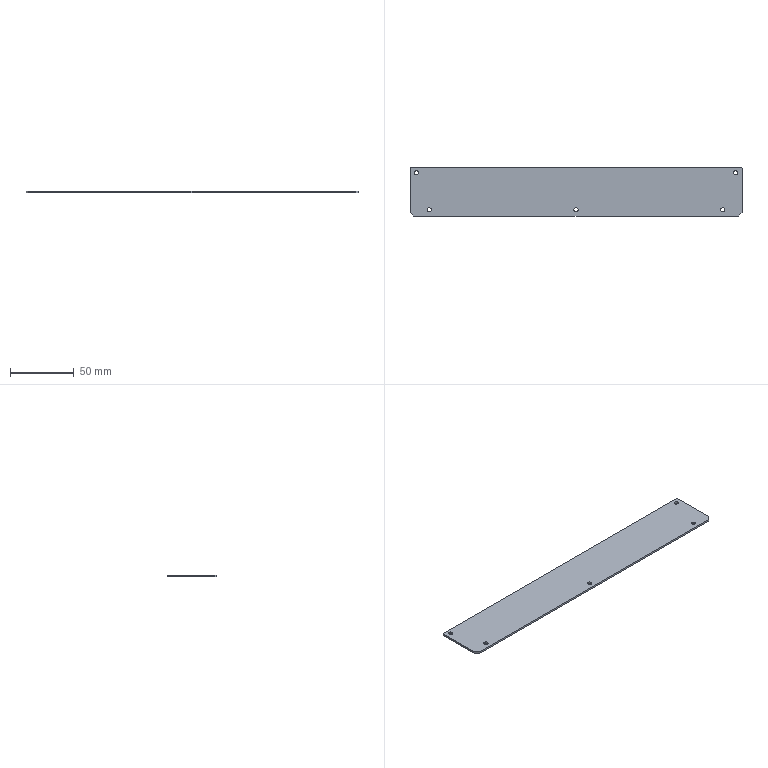Part | STEP file | PN_0066 Mount electronic clip s horizontal manipulator lower plate | 1 solid | 20 faces | box 260 x 38 x 1.5 mm | volume 14742 mm3 | cylinder 10 | plane 10 | commonest cylinder face diameters 3.3 x10
STEP:
#1=CARTESIAN_POINT('',(0.,0.,0.));
#2=DIRECTION('',(0.,0.,1.));
#3=DIRECTION('',(1.,0.,0.));
#4=AXIS2_PLACEMENT_3D('',#1,#2,#3);
#5=CARTESIAN_POINT('',(6.65,34.,-1.5));
#6=VERTEX_POINT('',#5);
#7=CARTESIAN_POINT('',(6.65,34.,0.));
#8=VERTEX_POINT('',#7);
#9=CARTESIAN_POINT('',(6.65,34.,0.));
#10=DIRECTION('',(0.,0.,1.));
#11=VECTOR('',#10,1.);
#12=LINE('',#9,#11);
#13=CARTESIAN_POINT('',(5.,34.,0.));
#14=DIRECTION('',(0.,0.,1.));
#15=DIRECTION('',(1.,0.,0.));
#16=AXIS2_PLACEMENT_3D('',#13,#14,#15);
#17=CYLINDRICAL_SURFACE('',#16,1.65);
#18=CARTESIAN_POINT('',(6.283,0.));
#19=DIRECTION('',(0.,1.));
#20=VECTOR('',#19,1.);
#21=LINE('',#18,#20);
#22=(GEOMETRIC_REPRESENTATION_CONTEXT(2)PARAMETRIC_REPRESENTATION_CONTEXT()REPRESENTATION_CONTEXT('',''));
#23=DEFINITIONAL_REPRESENTATION('',(#21),#22);
#24=PCURVE('',#17,#23);
#25=CARTESIAN_POINT('',(5.,34.,0.));
#26=DIRECTION('',(0.,0.,1.));
#27=DIRECTION('',(1.,0.,0.));
#28=AXIS2_PLACEMENT_3D('',#25,#26,#27);
#29=CYLINDRICAL_SURFACE('',#28,1.65);
#30=CARTESIAN_POINT('',(0.,0.));
#31=DIRECTION('',(0.,1.));
#32=VECTOR('',#31,1.);
#33=LINE('',#30,#32);
#34=(GEOMETRIC_REPRESENTATION_CONTEXT(2)PARAMETRIC_REPRESENTATION_CONTEXT()REPRESENTATION_CONTEXT('',''));
#35=DEFINITIONAL_REPRESENTATION('',(#33),#34);
#36=PCURVE('',#29,#35);
#37=SURFACE_CURVE('',#12,(#24,#36),.PCURVE_S1.);
#38=EDGE_CURVE('',#6,#8,#37,.T.);
#39=ORIENTED_EDGE('',*,*,#38,.T.);
#40=CARTESIAN_POINT('',(3.35,34.,0.));
#41=VERTEX_POINT('',#40);
#42=CARTESIAN_POINT('',(5.,34.,0.));
#43=DIRECTION('',(0.,0.,1.));
#44=DIRECTION('',(1.,0.,0.));
#45=AXIS2_PLACEMENT_3D('',#42,#43,#44);
#46=CIRCLE('',#45,1.65);
#47=CARTESIAN_POINT('',(0.,0.));
#48=DIRECTION('',(1.,0.));
#49=VECTOR('',#48,1.);
#50=LINE('',#47,#49);
#51=(GEOMETRIC_REPRESENTATION_CONTEXT(2)PARAMETRIC_REPRESENTATION_CONTEXT()REPRESENTATION_CONTEXT('',''));
#52=DEFINITIONAL_REPRESENTATION('',(#50),#51);
#53=PCURVE('',#17,#52);
#54=CARTESIAN_POINT('',(0.,0.,0.));
#55=DIRECTION('',(0.,0.,1.));
#56=DIRECTION('',(1.,0.,0.));
#57=AXIS2_PLACEMENT_3D('',#54,#55,#56);
#58=PLANE('',#57);
#59=CARTESIAN_POINT('',(5.,34.));
#60=DIRECTION('',(1.,0.));
#61=AXIS2_PLACEMENT_2D('',#59,#60);
#62=CIRCLE('',#61,1.65);
#63=(GEOMETRIC_REPRESENTATION_CONTEXT(2)PARAMETRIC_REPRESENTATION_CONTEXT()REPRESENTATION_CONTEXT('',''));
#64=DEFINITIONAL_REPRESENTATION('',(#62),#63);
#65=PCURVE('',#58,#64);
#66=SURFACE_CURVE('',#46,(#53,#65),.PCURVE_S1.);
#67=EDGE_CURVE('',#41,#8,#66,.T.);
#68=ORIENTED_EDGE('',*,*,#67,.F.);
#69=CARTESIAN_POINT('',(3.35,34.,-1.5));
#70=VERTEX_POINT('',#69);
#71=CARTESIAN_POINT('',(3.35,34.,0.));
#72=DIRECTION('',(0.,0.,1.));
#73=VECTOR('',#72,1.);
#74=LINE('',#71,#73);
#75=CARTESIAN_POINT('',(3.142,0.));
#76=DIRECTION('',(0.,1.));
#77=VECTOR('',#76,1.);
#78=LINE('',#75,#77);
#79=(GEOMETRIC_REPRESENTATION_CONTEXT(2)PARAMETRIC_REPRESENTATION_CONTEXT()REPRESENTATION_CONTEXT('',''));
#80=DEFINITIONAL_REPRESENTATION('',(#78),#79);
#81=PCURVE('',#17,#80);
#82=CARTESIAN_POINT('',(3.142,0.));
#83=DIRECTION('',(0.,1.));
#84=VECTOR('',#83,1.);
#85=LINE('',#82,#84);
#86=(GEOMETRIC_REPRESENTATION_CONTEXT(2)PARAMETRIC_REPRESENTATION_CONTEXT()REPRESENTATION_CONTEXT('',''));
#87=DEFINITIONAL_REPRESENTATION('',(#85),#86);
#88=PCURVE('',#29,#87);
#89=SURFACE_CURVE('',#74,(#81,#88),.PCURVE_S1.);
#90=EDGE_CURVE('',#70,#41,#89,.T.);
#91=ORIENTED_EDGE('',*,*,#90,.F.);
#92=CARTESIAN_POINT('',(5.,34.,-1.5));
#93=DIRECTION('',(0.,0.,1.));
#94=DIRECTION('',(1.,0.,0.));
#95=AXIS2_PLACEMENT_3D('',#92,#93,#94);
#96=CIRCLE('',#95,1.65);
#97=CARTESIAN_POINT('',(0.,-1.5));
#98=DIRECTION('',(1.,0.));
#99=VECTOR('',#98,1.);
#100=LINE('',#97,#99);
#101=(GEOMETRIC_REPRESENTATION_CONTEXT(2)PARAMETRIC_REPRESENTATION_CONTEXT()REPRESENTATION_CONTEXT('',''));
#102=DEFINITIONAL_REPRESENTATION('',(#100),#101);
#103=PCURVE('',#17,#102);
#104=CARTESIAN_POINT('',(0.,0.,-1.5));
#105=DIRECTION('',(0.,0.,1.));
#106=DIRECTION('',(1.,0.,0.));
#107=AXIS2_PLACEMENT_3D('',#104,#105,#106);
#108=PLANE('',#107);
#109=CARTESIAN_POINT('',(5.,34.));
#110=DIRECTION('',(1.,0.));
#111=AXIS2_PLACEMENT_2D('',#109,#110);
#112=CIRCLE('',#111,1.65);
#113=(GEOMETRIC_REPRESENTATION_CONTEXT(2)PARAMETRIC_REPRESENTATION_CONTEXT()REPRESENTATION_CONTEXT('',''));
#114=DEFINITIONAL_REPRESENTATION('',(#112),#113);
#115=PCURVE('',#108,#114);
#116=SURFACE_CURVE('',#96,(#103,#115),.PCURVE_S1.);
#117=EDGE_CURVE('',#70,#6,#116,.T.);
#118=ORIENTED_EDGE('',*,*,#117,.T.);
#119=EDGE_LOOP('',(#39,#68,#91,#118));
#120=FACE_BOUND('',#119,.F.);
#121=ADVANCED_FACE('',(#120),#17,.F.);
#122=CARTESIAN_POINT('',(16.65,5.,-1.5));
#123=VERTEX_POINT('',#122);
#124=CARTESIAN_POINT('',(16.65,5.,0.));
#125=VERTEX_POINT('',#124);
#126=CARTESIAN_POINT('',(16.65,5.,0.));
#127=DIRECTION('',(0.,0.,1.));
#128=VECTOR('',#127,1.);
#129=LINE('',#126,#128);
#130=CARTESIAN_POINT('',(15.,5.,0.));
#131=DIRECTION('',(0.,0.,1.));
#132=DIRECTION('',(1.,0.,0.));
#133=AXIS2_PLACEMENT_3D('',#130,#131,#132);
#134=CYLINDRICAL_SURFACE('',#133,1.65);
#135=CARTESIAN_POINT('',(6.283,0.));
#136=DIRECTION('',(0.,1.));
#137=VECTOR('',#136,1.);
#138=LINE('',#135,#137);
#139=(GEOMETRIC_REPRESENTATION_CONTEXT(2)PARAMETRIC_REPRESENTATION_CONTEXT()REPRESENTATION_CONTEXT('',''));
#140=DEFINITIONAL_REPRESENTATION('',(#138),#139);
#141=PCURVE('',#134,#140);
#142=CARTESIAN_POINT('',(15.,5.,0.));
#143=DIRECTION('',(0.,0.,1.));
#144=DIRECTION('',(1.,0.,0.));
#145=AXIS2_PLACEMENT_3D('',#142,#143,#144);
#146=CYLINDRICAL_SURFACE('',#145,1.65);
#147=CARTESIAN_POINT('',(0.,0.));
#148=DIRECTION('',(0.,1.));
#149=VECTOR('',#148,1.);
#150=LINE('',#147,#149);
#151=(GEOMETRIC_REPRESENTATION_CONTEXT(2)PARAMETRIC_REPRESENTATION_CONTEXT()REPRESENTATION_CONTEXT('',''));
#152=DEFINITIONAL_REPRESENTATION('',(#150),#151);
#153=PCURVE('',#146,#152);
#154=SURFACE_CURVE('',#129,(#141,#153),.PCURVE_S1.);
#155=EDGE_CURVE('',#123,#125,#154,.T.);
#156=ORIENTED_EDGE('',*,*,#155,.T.);
#157=CARTESIAN_POINT('',(13.35,5.,0.));
#158=VERTEX_POINT('',#157);
#159=CARTESIAN_POINT('',(15.,5.,0.));
#160=DIRECTION('',(0.,0.,1.));
#161=DIRECTION('',(1.,0.,0.));
#162=AXIS2_PLACEMENT_3D('',#159,#160,#161);
#163=CIRCLE('',#162,1.65);
#164=CARTESIAN_POINT('',(0.,0.));
#165=DIRECTION('',(1.,0.));
#166=VECTOR('',#165,1.);
#167=LINE('',#164,#166);
#168=(GEOMETRIC_REPRESENTATION_CONTEXT(2)PARAMETRIC_REPRESENTATION_CONTEXT()REPRESENTATION_CONTEXT('',''));
#169=DEFINITIONAL_REPRESENTATION('',(#167),#168);
#170=PCURVE('',#134,#169);
#171=CARTESIAN_POINT('',(15.,5.));
#172=DIRECTION('',(1.,0.));
#173=AXIS2_PLACEMENT_2D('',#171,#172);
#174=CIRCLE('',#173,1.65);
#175=(GEOMETRIC_REPRESENTATION_CONTEXT(2)PARAMETRIC_REPRESENTATION_CONTEXT()REPRESENTATION_CONTEXT('',''));
#176=DEFINITIONAL_REPRESENTATION('',(#174),#175);
#177=PCURVE('',#58,#176);
#178=SURFACE_CURVE('',#163,(#170,#177),.PCURVE_S1.);
#179=EDGE_CURVE('',#158,#125,#178,.T.);
#180=ORIENTED_EDGE('',*,*,#179,.F.);
#181=CARTESIAN_POINT('',(13.35,5.,-1.5));
#182=VERTEX_POINT('',#181);
#183=CARTESIAN_POINT('',(13.35,5.,0.));
#184=DIRECTION('',(0.,0.,1.));
#185=VECTOR('',#184,1.);
#186=LINE('',#183,#185);
#187=CARTESIAN_POINT('',(3.142,0.));
#188=DIRECTION('',(0.,1.));
#189=VECTOR('',#188,1.);
#190=LINE('',#187,#189);
#191=(GEOMETRIC_REPRESENTATION_CONTEXT(2)PARAMETRIC_REPRESENTATION_CONTEXT()REPRESENTATION_CONTEXT('',''));
#192=DEFINITIONAL_REPRESENTATION('',(#190),#191);
#193=PCURVE('',#134,#192);
#194=CARTESIAN_POINT('',(3.142,0.));
#195=DIRECTION('',(0.,1.));
#196=VECTOR('',#195,1.);
#197=LINE('',#194,#196);
#198=(GEOMETRIC_REPRESENTATION_CONTEXT(2)PARAMETRIC_REPRESENTATION_CONTEXT()REPRESENTATION_CONTEXT('',''));
#199=DEFINITIONAL_REPRESENTATION('',(#197),#198);
#200=PCURVE('',#146,#199);
#201=SURFACE_CURVE('',#186,(#193,#200),.PCURVE_S1.);
#202=EDGE_CURVE('',#182,#158,#201,.T.);
#203=ORIENTED_EDGE('',*,*,#202,.F.);
#204=CARTESIAN_POINT('',(15.,5.,-1.5));
#205=DIRECTION('',(0.,0.,1.));
#206=DIRECTION('',(1.,0.,0.));
#207=AXIS2_PLACEMENT_3D('',#204,#205,#206);
#208=CIRCLE('',#207,1.65);
#209=CARTESIAN_POINT('',(0.,-1.5));
#210=DIRECTION('',(1.,0.));
#211=VECTOR('',#210,1.);
#212=LINE('',#209,#211);
#213=(GEOMETRIC_REPRESENTATION_CONTEXT(2)PARAMETRIC_REPRESENTATION_CONTEXT()REPRESENTATION_CONTEXT('',''));
#214=DEFINITIONAL_REPRESENTATION('',(#212),#213);
#215=PCURVE('',#134,#214);
#216=CARTESIAN_POINT('',(15.,5.));
#217=DIRECTION('',(1.,0.));
#218=AXIS2_PLACEMENT_2D('',#216,#217);
#219=CIRCLE('',#218,1.65);
#220=(GEOMETRIC_REPRESENTATION_CONTEXT(2)PARAMETRIC_REPRESENTATION_CONTEXT()REPRESENTATION_CONTEXT('',''));
#221=DEFINITIONAL_REPRESENTATION('',(#219),#220);
#222=PCURVE('',#108,#221);
#223=SURFACE_CURVE('',#208,(#215,#222),.PCURVE_S1.);
#224=EDGE_CURVE('',#182,#123,#223,.T.);
#225=ORIENTED_EDGE('',*,*,#224,.T.);
#226=EDGE_LOOP('',(#156,#180,#203,#225));
#227=FACE_BOUND('',#226,.F.);
#228=ADVANCED_FACE('',(#227),#134,.F.);
#229=CARTESIAN_POINT('',(256.65,34.,-1.5));
#230=VERTEX_POINT('',#229);
#231=CARTESIAN_POINT('',(256.65,34.,0.));
#232=VERTEX_POINT('',#231);
#233=CARTESIAN_POINT('',(256.65,34.,0.));
#234=DIRECTION('',(0.,0.,1.));
#235=VECTOR('',#234,1.);
#236=LINE('',#233,#235);
#237=CARTESIAN_POINT('',(255.,34.,0.));
#238=DIRECTION('',(0.,0.,1.));
#239=DIRECTION('',(1.,0.,0.));
#240=AXIS2_PLACEMENT_3D('',#237,#238,#239);
#241=CYLINDRICAL_SURFACE('',#240,1.65);
#242=CARTESIAN_POINT('',(6.283,0.));
#243=DIRECTION('',(0.,1.));
#244=VECTOR('',#243,1.);
#245=LINE('',#242,#244);
#246=(GEOMETRIC_REPRESENTATION_CONTEXT(2)PARAMETRIC_REPRESENTATION_CONTEXT()REPRESENTATION_CONTEXT('',''));
#247=DEFINITIONAL_REPRESENTATION('',(#245),#246);
#248=PCURVE('',#241,#247);
#249=CARTESIAN_POINT('',(255.,34.,0.));
#250=DIRECTION('',(0.,0.,1.));
#251=DIRECTION('',(1.,0.,0.));
#252=AXIS2_PLACEMENT_3D('',#249,#250,#251);
#253=CYLINDRICAL_SURFACE('',#252,1.65);
#254=CARTESIAN_POINT('',(0.,0.));
#255=DIRECTION('',(0.,1.));
#256=VECTOR('',#255,1.);
#257=LINE('',#254,#256);
#258=(GEOMETRIC_REPRESENTATION_CONTEXT(2)PARAMETRIC_REPRESENTATION_CONTEXT()REPRESENTATION_CONTEXT('',''));
#259=DEFINITIONAL_REPRESENTATION('',(#257),#258);
#260=PCURVE('',#253,#259);
#261=SURFACE_CURVE('',#236,(#248,#260),.PCURVE_S1.);
#262=EDGE_CURVE('',#230,#232,#261,.T.);
#263=ORIENTED_EDGE('',*,*,#262,.T.);
#264=CARTESIAN_POINT('',(253.35,34.,0.));
#265=VERTEX_POINT('',#264);
#266=CARTESIAN_POINT('',(255.,34.,0.));
#267=DIRECTION('',(0.,0.,1.));
#268=DIRECTION('',(1.,0.,0.));
#269=AXIS2_PLACEMENT_3D('',#266,#267,#268);
#270=CIRCLE('',#269,1.65);
#271=CARTESIAN_POINT('',(0.,0.));
#272=DIRECTION('',(1.,0.));
#273=VECTOR('',#272,1.);
#274=LINE('',#271,#273);
#275=(GEOMETRIC_REPRESENTATION_CONTEXT(2)PARAMETRIC_REPRESENTATION_CONTEXT()REPRESENTATION_CONTEXT('',''));
#276=DEFINITIONAL_REPRESENTATION('',(#274),#275);
#277=PCURVE('',#241,#276);
#278=CARTESIAN_POINT('',(255.,34.));
#279=DIRECTION('',(1.,0.));
#280=AXIS2_PLACEMENT_2D('',#278,#279);
#281=CIRCLE('',#280,1.65);
#282=(GEOMETRIC_REPRESENTATION_CONTEXT(2)PARAMETRIC_REPRESENTATION_CONTEXT()REPRESENTATION_CONTEXT('',''));
#283=DEFINITIONAL_REPRESENTATION('',(#281),#282);
#284=PCURVE('',#58,#283);
#285=SURFACE_CURVE('',#270,(#277,#284),.PCURVE_S1.);
#286=EDGE_CURVE('',#265,#232,#285,.T.);
#287=ORIENTED_EDGE('',*,*,#286,.F.);
#288=CARTESIAN_POINT('',(253.35,34.,-1.5));
#289=VERTEX_POINT('',#288);
#290=CARTESIAN_POINT('',(253.35,34.,0.));
#291=DIRECTION('',(0.,0.,1.));
#292=VECTOR('',#291,1.);
#293=LINE('',#290,#292);
#294=CARTESIAN_POINT('',(3.142,0.));
#295=DIRECTION('',(0.,1.));
#296=VECTOR('',#295,1.);
#297=LINE('',#294,#296);
#298=(GEOMETRIC_REPRESENTATION_CONTEXT(2)PARAMETRIC_REPRESENTATION_CONTEXT()REPRESENTATION_CONTEXT('',''));
#299=DEFINITIONAL_REPRESENTATION('',(#297),#298);
#300=PCURVE('',#241,#299);
#301=CARTESIAN_POINT('',(3.142,0.));
#302=DIRECTION('',(0.,1.));
#303=VECTOR('',#302,1.);
#304=LINE('',#301,#303);
#305=(GEOMETRIC_REPRESENTATION_CONTEXT(2)PARAMETRIC_REPRESENTATION_CONTEXT()REPRESENTATION_CONTEXT('',''));
#306=DEFINITIONAL_REPRESENTATION('',(#304),#305);
#307=PCURVE('',#253,#306);
#308=SURFACE_CURVE('',#293,(#300,#307),.PCURVE_S1.);
#309=EDGE_CURVE('',#289,#265,#308,.T.);
#310=ORIENTED_EDGE('',*,*,#309,.F.);
#311=CARTESIAN_POINT('',(255.,34.,-1.5));
#312=DIRECTION('',(0.,0.,1.));
#313=DIRECTION('',(1.,0.,0.));
#314=AXIS2_PLACEMENT_3D('',#311,#312,#313);
#315=CIRCLE('',#314,1.65);
#316=CARTESIAN_POINT('',(0.,-1.5));
#317=DIRECTION('',(1.,0.));
#318=VECTOR('',#317,1.);
#319=LINE('',#316,#318);
#320=(GEOMETRIC_REPRESENTATION_CONTEXT(2)PARAMETRIC_REPRESENTATION_CONTEXT()REPRESENTATION_CONTEXT('',''));
#321=DEFINITIONAL_REPRESENTATION('',(#319),#320);
#322=PCURVE('',#241,#321);
#323=CARTESIAN_POINT('',(255.,34.));
#324=DIRECTION('',(1.,0.));
#325=AXIS2_PLACEMENT_2D('',#323,#324);
#326=CIRCLE('',#325,1.65);
#327=(GEOMETRIC_REPRESENTATION_CONTEXT(2)PARAMETRIC_REPRESENTATION_CONTEXT()REPRESENTATION_CONTEXT('',''));
#328=DEFINITIONAL_REPRESENTATION('',(#326),#327);
#329=PCURVE('',#108,#328);
#330=SURFACE_CURVE('',#315,(#322,#329),.PCURVE_S1.);
#331=EDGE_CURVE('',#289,#230,#330,.T.);
#332=ORIENTED_EDGE('',*,*,#331,.T.);
#333=EDGE_LOOP('',(#263,#287,#310,#332));
#334=FACE_BOUND('',#333,.F.);
#335=ADVANCED_FACE('',(#334),#241,.F.);
#336=CARTESIAN_POINT('',(246.65,5.,-1.5));
#337=VERTEX_POINT('',#336);
#338=CARTESIAN_POINT('',(246.65,5.,0.));
#339=VERTEX_POINT('',#338);
#340=CARTESIAN_POINT('',(246.65,5.,0.));
#341=DIRECTION('',(0.,0.,1.));
#342=VECTOR('',#341,1.);
#343=LINE('',#340,#342);
#344=CARTESIAN_POINT('',(245.,5.,0.));
#345=DIRECTION('',(0.,0.,1.));
#346=DIRECTION('',(1.,0.,0.));
#347=AXIS2_PLACEMENT_3D('',#344,#345,#346);
#348=CYLINDRICAL_SURFACE('',#347,1.65);
#349=CARTESIAN_POINT('',(6.283,0.));
#350=DIRECTION('',(0.,1.));
#351=VECTOR('',#350,1.);
#352=LINE('',#349,#351);
#353=(GEOMETRIC_REPRESENTATION_CONTEXT(2)PARAMETRIC_REPRESENTATION_CONTEXT()REPRESENTATION_CONTEXT('',''));
#354=DEFINITIONAL_REPRESENTATION('',(#352),#353);
#355=PCURVE('',#348,#354);
#356=CARTESIAN_POINT('',(245.,5.,0.));
#357=DIRECTION('',(0.,0.,1.));
#358=DIRECTION('',(1.,0.,0.));
#359=AXIS2_PLACEMENT_3D('',#356,#357,#358);
#360=CYLINDRICAL_SURFACE('',#359,1.65);
#361=CARTESIAN_POINT('',(0.,0.));
#362=DIRECTION('',(0.,1.));
#363=VECTOR('',#362,1.);
#364=LINE('',#361,#363);
#365=(GEOMETRIC_REPRESENTATION_CONTEXT(2)PARAMETRIC_REPRESENTATION_CONTEXT()REPRESENTATION_CONTEXT('',''));
#366=DEFINITIONAL_REPRESENTATION('',(#364),#365);
#367=PCURVE('',#360,#366);
#368=SURFACE_CURVE('',#343,(#355,#367),.PCURVE_S1.);
#369=EDGE_CURVE('',#337,#339,#368,.T.);
#370=ORIENTED_EDGE('',*,*,#369,.T.);
#371=CARTESIAN_POINT('',(243.35,5.,0.));
#372=VERTEX_POINT('',#371);
#373=CARTESIAN_POINT('',(245.,5.,0.));
#374=DIRECTION('',(0.,0.,1.));
#375=DIRECTION('',(1.,0.,0.));
#376=AXIS2_PLACEMENT_3D('',#373,#374,#375);
#377=CIRCLE('',#376,1.65);
#378=CARTESIAN_POINT('',(0.,0.));
#379=DIRECTION('',(1.,0.));
#380=VECTOR('',#379,1.);
#381=LINE('',#378,#380);
#382=(GEOMETRIC_REPRESENTATION_CONTEXT(2)PARAMETRIC_REPRESENTATION_CONTEXT()REPRESENTATION_CONTEXT('',''));
#383=DEFINITIONAL_REPRESENTATION('',(#381),#382);
#384=PCURVE('',#348,#383);
#385=CARTESIAN_POINT('',(245.,5.));
#386=DIRECTION('',(1.,0.));
#387=AXIS2_PLACEMENT_2D('',#385,#386);
#388=CIRCLE('',#387,1.65);
#389=(GEOMETRIC_REPRESENTATION_CONTEXT(2)PARAMETRIC_REPRESENTATION_CONTEXT()REPRESENTATION_CONTEXT('',''));
#390=DEFINITIONAL_REPRESENTATION('',(#388),#389);
#391=PCURVE('',#58,#390);
#392=SURFACE_CURVE('',#377,(#384,#391),.PCURVE_S1.);
#393=EDGE_CURVE('',#372,#339,#392,.T.);
#394=ORIENTED_EDGE('',*,*,#393,.F.);
#395=CARTESIAN_POINT('',(243.35,5.,-1.5));
#396=VERTEX_POINT('',#395);
#397=CARTESIAN_POINT('',(243.35,5.,0.));
#398=DIRECTION('',(0.,0.,1.));
#399=VECTOR('',#398,1.);
#400=LINE('',#397,#399);
#401=CARTESIAN_POINT('',(3.142,0.));
#402=DIRECTION('',(0.,1.));
#403=VECTOR('',#402,1.);
#404=LINE('',#401,#403);
#405=(GEOMETRIC_REPRESENTATION_CONTEXT(2)PARAMETRIC_REPRESENTATION_CONTEXT()REPRESENTATION_CONTEXT('',''));
#406=DEFINITIONAL_REPRESENTATION('',(#404),#405);
#407=PCURVE('',#348,#406);
#408=CARTESIAN_POINT('',(3.142,0.));
#409=DIRECTION('',(0.,1.));
#410=VECTOR('',#409,1.);
#411=LINE('',#408,#410);
#412=(GEOMETRIC_REPRESENTATION_CONTEXT(2)PARAMETRIC_REPRESENTATION_CONTEXT()REPRESENTATION_CONTEXT('',''));
#413=DEFINITIONAL_REPRESENTATION('',(#411),#412);
#414=PCURVE('',#360,#413);
#415=SURFACE_CURVE('',#400,(#407,#414),.PCURVE_S1.);
#416=EDGE_CURVE('',#396,#372,#415,.T.);
#417=ORIENTED_EDGE('',*,*,#416,.F.);
#418=CARTESIAN_POINT('',(245.,5.,-1.5));
#419=DIRECTION('',(0.,0.,1.));
#420=DIRECTION('',(1.,0.,0.));
#421=AXIS2_PLACEMENT_3D('',#418,#419,#420);
#422=CIRCLE('',#421,1.65);
#423=CARTESIAN_POINT('',(0.,-1.5));
#424=DIRECTION('',(1.,0.));
#425=VECTOR('',#424,1.);
#426=LINE('',#423,#425);
#427=(GEOMETRIC_REPRESENTATION_CONTEXT(2)PARAMETRIC_REPRESENTATION_CONTEXT()REPRESENTATION_CONTEXT('',''));
#428=DEFINITIONAL_REPRESENTATION('',(#426),#427);
#429=PCURVE('',#348,#428);
#430=CARTESIAN_POINT('',(245.,5.));
#431=DIRECTION('',(1.,0.));
#432=AXIS2_PLACEMENT_2D('',#430,#431);
#433=CIRCLE('',#432,1.65);
#434=(GEOMETRIC_REPRESENTATION_CONTEXT(2)PARAMETRIC_REPRESENTATION_CONTEXT()REPRESENTATION_CONTEXT('',''));
#435=DEFINITIONAL_REPRESENTATION('',(#433),#434);
#436=PCURVE('',#108,#435);
#437=SURFACE_CURVE('',#422,(#429,#436),.PCURVE_S1.);
#438=EDGE_CURVE('',#396,#337,#437,.T.);
#439=ORIENTED_EDGE('',*,*,#438,.T.);
#440=EDGE_LOOP('',(#370,#394,#417,#439));
#441=FACE_BOUND('',#440,.F.);
#442=ADVANCED_FACE('',(#441),#348,.F.);
#443=CARTESIAN_POINT('',(131.65,5.,-1.5));
#444=VERTEX_POINT('',#443);
#445=CARTESIAN_POINT('',(131.65,5.,0.));
#446=VERTEX_POINT('',#445);
#447=CARTESIAN_POINT('',(131.65,5.,0.));
#448=DIRECTION('',(0.,0.,1.));
#449=VECTOR('',#448,1.);
#450=LINE('',#447,#449);
#451=CARTESIAN_POINT('',(130.,5.,0.));
#452=DIRECTION('',(0.,0.,1.));
#453=DIRECTION('',(1.,0.,0.));
#454=AXIS2_PLACEMENT_3D('',#451,#452,#453);
#455=CYLINDRICAL_SURFACE('',#454,1.65);
#456=CARTESIAN_POINT('',(6.283,0.));
#457=DIRECTION('',(0.,1.));
#458=VECTOR('',#457,1.);
#459=LINE('',#456,#458);
#460=(GEOMETRIC_REPRESENTATION_CONTEXT(2)PARAMETRIC_REPRESENTATION_CONTEXT()REPRESENTATION_CONTEXT('',''));
#461=DEFINITIONAL_REPRESENTATION('',(#459),#460);
#462=PCURVE('',#455,#461);
#463=CARTESIAN_POINT('',(130.,5.,0.));
#464=DIRECTION('',(0.,0.,1.));
#465=DIRECTION('',(1.,0.,0.));
#466=AXIS2_PLACEMENT_3D('',#463,#464,#465);
#467=CYLINDRICAL_SURFACE('',#466,1.65);
#468=CARTESIAN_POINT('',(0.,0.));
#469=DIRECTION('',(0.,1.));
#470=VECTOR('',#469,1.);
#471=LINE('',#468,#470);
#472=(GEOMETRIC_REPRESENTATION_CONTEXT(2)PARAMETRIC_REPRESENTATION_CONTEXT()REPRESENTATION_CONTEXT('',''));
#473=DEFINITIONAL_REPRESENTATION('',(#471),#472);
#474=PCURVE('',#467,#473);
#475=SURFACE_CURVE('',#450,(#462,#474),.PCURVE_S1.);
#476=EDGE_CURVE('',#444,#446,#475,.T.);
#477=ORIENTED_EDGE('',*,*,#476,.T.);
#478=CARTESIAN_POINT('',(128.35,5.,0.));
#479=VERTEX_POINT('',#478);
#480=CARTESIAN_POINT('',(130.,5.,0.));
#481=DIRECTION('',(0.,0.,1.));
#482=DIRECTION('',(1.,0.,0.));
#483=AXIS2_PLACEMENT_3D('',#480,#481,#482);
#484=CIRCLE('',#483,1.65);
#485=CARTESIAN_POINT('',(0.,0.));
#486=DIRECTION('',(1.,0.));
#487=VECTOR('',#486,1.);
#488=LINE('',#485,#487);
#489=(GEOMETRIC_REPRESENTATION_CONTEXT(2)PARAMETRIC_REPRESENTATION_CONTEXT()REPRESENTATION_CONTEXT('',''));
#490=DEFINITIONAL_REPRESENTATION('',(#488),#489);
#491=PCURVE('',#455,#490);
#492=CARTESIAN_POINT('',(130.,5.));
#493=DIRECTION('',(1.,0.));
#494=AXIS2_PLACEMENT_2D('',#492,#493);
#495=CIRCLE('',#494,1.65);
#496=(GEOMETRIC_REPRESENTATION_CONTEXT(2)PARAMETRIC_REPRESENTATION_CONTEXT()REPRESENTATION_CONTEXT('',''));
#497=DEFINITIONAL_REPRESENTATION('',(#495),#496);
#498=PCURVE('',#58,#497);
#499=SURFACE_CURVE('',#484,(#491,#498),.PCURVE_S1.);
#500=EDGE_CURVE('',#479,#446,#499,.T.);
#501=ORIENTED_EDGE('',*,*,#500,.F.);
#502=CARTESIAN_POINT('',(128.35,5.,-1.5));
#503=VERTEX_POINT('',#502);
#504=CARTESIAN_POINT('',(128.35,5.,0.));
#505=DIRECTION('',(0.,0.,1.));
#506=VECTOR('',#505,1.);
#507=LINE('',#504,#506);
#508=CARTESIAN_POINT('',(3.142,0.));
#509=DIRECTION('',(0.,1.));
#510=VECTOR('',#509,1.);
#511=LINE('',#508,#510);
#512=(GEOMETRIC_REPRESENTATION_CONTEXT(2)PARAMETRIC_REPRESENTATION_CONTEXT()REPRESENTATION_CONTEXT('',''));
#513=DEFINITIONAL_REPRESENTATION('',(#511),#512);
#514=PCURVE('',#455,#513);
#515=CARTESIAN_POINT('',(3.142,0.));
#516=DIRECTION('',(0.,1.));
#517=VECTOR('',#516,1.);
#518=LINE('',#515,#517);
#519=(GEOMETRIC_REPRESENTATION_CONTEXT(2)PARAMETRIC_REPRESENTATION_CONTEXT()REPRESENTATION_CONTEXT('',''));
#520=DEFINITIONAL_REPRESENTATION('',(#518),#519);
#521=PCURVE('',#467,#520);
#522=SURFACE_CURVE('',#507,(#514,#521),.PCURVE_S1.);
#523=EDGE_CURVE('',#503,#479,#522,.T.);
#524=ORIENTED_EDGE('',*,*,#523,.F.);
#525=CARTESIAN_POINT('',(130.,5.,-1.5));
#526=DIRECTION('',(0.,0.,1.));
#527=DIRECTION('',(1.,0.,0.));
#528=AXIS2_PLACEMENT_3D('',#525,#526,#527);
#529=CIRCLE('',#528,1.65);
#530=CARTESIAN_POINT('',(0.,-1.5));
#531=DIRECTION('',(1.,0.));
#532=VECTOR('',#531,1.);
#533=LINE('',#530,#532);
#534=(GEOMETRIC_REPRESENTATION_CONTEXT(2)PARAMETRIC_REPRESENTATION_CONTEXT()REPRESENTATION_CONTEXT('',''));
#535=DEFINITIONAL_REPRESENTATION('',(#533),#534);
#536=PCURVE('',#455,#535);
#537=CARTESIAN_POINT('',(130.,5.));
#538=DIRECTION('',(1.,0.));
#539=AXIS2_PLACEMENT_2D('',#537,#538);
#540=CIRCLE('',#539,1.65);
#541=(GEOMETRIC_REPRESENTATION_CONTEXT(2)PARAMETRIC_REPRESENTATION_CONTEXT()REPRESENTATION_CONTEXT('',''));
#542=DEFINITIONAL_REPRESENTATION('',(#540),#541);
#543=PCURVE('',#108,#542);
#544=SURFACE_CURVE('',#529,(#536,#543),.PCURVE_S1.);
#545=EDGE_CURVE('',#503,#444,#544,.T.);
#546=ORIENTED_EDGE('',*,*,#545,.T.);
#547=EDGE_LOOP('',(#477,#501,#524,#546));
#548=FACE_BOUND('',#547,.F.);
#549=ADVANCED_FACE('',(#548),#455,.F.);
#550=CARTESIAN_POINT('',(0.,37.5,-1.5));
#551=VERTEX_POINT('',#550);
#552=CARTESIAN_POINT('',(0.,3.,-1.5));
#553=VERTEX_POINT('',#552);
#554=CARTESIAN_POINT('',(0.,38.,-1.5));
#555=DIRECTION('',(0.,-1.,0.));
#556=VECTOR('',#555,1.);
#557=LINE('',#554,#556);
#558=CARTESIAN_POINT('',(0.,38.,-1.5));
#559=DIRECTION('',(-1.,0.,0.));
#560=DIRECTION('',(0.,-1.,0.));
#561=AXIS2_PLACEMENT_3D('',#558,#559,#560);
#562=PLANE('',#561);
#563=CARTESIAN_POINT('',(0.,0.));
#564=DIRECTION('',(1.,0.));
#565=VECTOR('',#564,1.);
#566=LINE('',#563,#565);
#567=(GEOMETRIC_REPRESENTATION_CONTEXT(2)PARAMETRIC_REPRESENTATION_CONTEXT()REPRESENTATION_CONTEXT('',''));
#568=DEFINITIONAL_REPRESENTATION('',(#566),#567);
#569=PCURVE('',#562,#568);
#570=CARTESIAN_POINT('',(0.,38.));
#571=DIRECTION('',(0.,-1.));
#572=VECTOR('',#571,1.);
#573=LINE('',#570,#572);
#574=(GEOMETRIC_REPRESENTATION_CONTEXT(2)PARAMETRIC_REPRESENTATION_CONTEXT()REPRESENTATION_CONTEXT('',''));
#575=DEFINITIONAL_REPRESENTATION('',(#573),#574);
#576=PCURVE('',#108,#575);
#577=SURFACE_CURVE('',#557,(#569,#576),.PCURVE_S1.);
#578=EDGE_CURVE('',#551,#553,#577,.T.);
#579=ORIENTED_EDGE('',*,*,#578,.T.);
#580=CARTESIAN_POINT('',(0.,3.,0.));
#581=VERTEX_POINT('',#580);
#582=CARTESIAN_POINT('',(0.,3.,-1.5));
#583=DIRECTION('',(0.,0.,1.));
#584=VECTOR('',#583,1.);
#585=LINE('',#582,#584);
#586=CARTESIAN_POINT('',(35.,0.));
#587=DIRECTION('',(0.,1.));
#588=VECTOR('',#587,1.);
#589=LINE('',#586,#588);
#590=(GEOMETRIC_REPRESENTATION_CONTEXT(2)PARAMETRIC_REPRESENTATION_CONTEXT()REPRESENTATION_CONTEXT('',''));
#591=DEFINITIONAL_REPRESENTATION('',(#589),#590);
#592=PCURVE('',#562,#591);
#593=CARTESIAN_POINT('',(0.,3.,-1.5));
#594=DIRECTION('',(0.7071,0.7071,0.));
#595=DIRECTION('',(-0.7071,0.7071,0.));
#596=AXIS2_PLACEMENT_3D('',#593,#594,#595);
#597=PLANE('',#596);
#598=CARTESIAN_POINT('',(0.,0.));
#599=DIRECTION('',(0.,1.));
#600=VECTOR('',#599,1.);
#601=LINE('',#598,#600);
#602=(GEOMETRIC_REPRESENTATION_CONTEXT(2)PARAMETRIC_REPRESENTATION_CONTEXT()REPRESENTATION_CONTEXT('',''));
#603=DEFINITIONAL_REPRESENTATION('',(#601),#602);
#604=PCURVE('',#597,#603);
#605=SURFACE_CURVE('',#585,(#592,#604),.PCURVE_S1.);
#606=EDGE_CURVE('',#553,#581,#605,.T.);
#607=ORIENTED_EDGE('',*,*,#606,.T.);
#608=CARTESIAN_POINT('',(0.,37.5,0.));
#609=VERTEX_POINT('',#608);
#610=CARTESIAN_POINT('',(0.,38.,0.));
#611=DIRECTION('',(0.,-1.,0.));
#612=VECTOR('',#611,1.);
#613=LINE('',#610,#612);
#614=CARTESIAN_POINT('',(0.,1.5));
#615=DIRECTION('',(1.,0.));
#616=VECTOR('',#615,1.);
#617=LINE('',#614,#616);
#618=(GEOMETRIC_REPRESENTATION_CONTEXT(2)PARAMETRIC_REPRESENTATION_CONTEXT()REPRESENTATION_CONTEXT('',''));
#619=DEFINITIONAL_REPRESENTATION('',(#617),#618);
#620=PCURVE('',#562,#619);
#621=CARTESIAN_POINT('',(0.,38.));
#622=DIRECTION('',(0.,-1.));
#623=VECTOR('',#622,1.);
#624=LINE('',#621,#623);
#625=(GEOMETRIC_REPRESENTATION_CONTEXT(2)PARAMETRIC_REPRESENTATION_CONTEXT()REPRESENTATION_CONTEXT('',''));
#626=DEFINITIONAL_REPRESENTATION('',(#624),#625);
#627=PCURVE('',#58,#626);
#628=SURFACE_CURVE('',#613,(#620,#627),.PCURVE_S1.);
#629=EDGE_CURVE('',#609,#581,#628,.T.);
#630=ORIENTED_EDGE('',*,*,#629,.F.);
#631=CARTESIAN_POINT('',(0.,37.5,-1.5));
#632=DIRECTION('',(0.,0.,-1.));
#633=VECTOR('',#632,1.);
#634=LINE('',#631,#633);
#635=CARTESIAN_POINT('',(0.5,0.));
#636=DIRECTION('',(0.,-1.));
#637=VECTOR('',#636,1.);
#638=LINE('',#635,#637);
#639=(GEOMETRIC_REPRESENTATION_CONTEXT(2)PARAMETRIC_REPRESENTATION_CONTEXT()REPRESENTATION_CONTEXT('',''));
#640=DEFINITIONAL_REPRESENTATION('',(#638),#639);
#641=PCURVE('',#562,#640);
#642=CARTESIAN_POINT('',(0.5,38.,-1.5));
#643=DIRECTION('',(0.7071,-0.7071,0.));
#644=DIRECTION('',(0.7071,0.7071,0.));
#645=AXIS2_PLACEMENT_3D('',#642,#643,#644);
#646=PLANE('',#645);
#647=CARTESIAN_POINT('',(-0.7071,0.));
#648=DIRECTION('',(0.,-1.));
#649=VECTOR('',#648,1.);
#650=LINE('',#647,#649);
#651=(GEOMETRIC_REPRESENTATION_CONTEXT(2)PARAMETRIC_REPRESENTATION_CONTEXT()REPRESENTATION_CONTEXT('',''));
#652=DEFINITIONAL_REPRESENTATION('',(#650),#651);
#653=PCURVE('',#646,#652);
#654=SURFACE_CURVE('',#634,(#641,#653),.PCURVE_S1.);
#655=EDGE_CURVE('',#609,#551,#654,.T.);
#656=ORIENTED_EDGE('',*,*,#655,.T.);
#657=EDGE_LOOP('',(#579,#607,#630,#656));
#658=FACE_BOUND('',#657,.T.);
#659=ADVANCED_FACE('',(#658),#562,.T.);
#660=CARTESIAN_POINT('',(259.5,38.,-1.5));
#661=VERTEX_POINT('',#660);
#662=CARTESIAN_POINT('',(0.5,38.,-1.5));
#663=VERTEX_POINT('',#662);
#664=CARTESIAN_POINT('',(0.,38.,-1.5));
#665=DIRECTION('',(-1.,0.,0.));
#666=VECTOR('',#665,1.);
#667=LINE('',#664,#666);
#668=CARTESIAN_POINT('',(0.,38.,-1.5));
#669=DIRECTION('',(0.,1.,0.));
#670=DIRECTION('',(0.,0.,1.));
#671=AXIS2_PLACEMENT_3D('',#668,#669,#670);
#672=PLANE('',#671);
#673=CARTESIAN_POINT('',(0.,0.));
#674=DIRECTION('',(0.,-1.));
#675=VECTOR('',#674,1.);
#676=LINE('',#673,#675);
#677=(GEOMETRIC_REPRESENTATION_CONTEXT(2)PARAMETRIC_REPRESENTATION_CONTEXT()REPRESENTATION_CONTEXT('',''));
#678=DEFINITIONAL_REPRESENTATION('',(#676),#677);
#679=PCURVE('',#672,#678);
#680=CARTESIAN_POINT('',(0.,38.));
#681=DIRECTION('',(-1.,0.));
#682=VECTOR('',#681,1.);
#683=LINE('',#680,#682);
#684=(GEOMETRIC_REPRESENTATION_CONTEXT(2)PARAMETRIC_REPRESENTATION_CONTEXT()REPRESENTATION_CONTEXT('',''));
#685=DEFINITIONAL_REPRESENTATION('',(#683),#684);
#686=PCURVE('',#108,#685);
#687=SURFACE_CURVE('',#667,(#679,#686),.PCURVE_S1.);
#688=EDGE_CURVE('',#661,#663,#687,.T.);
#689=ORIENTED_EDGE('',*,*,#688,.T.);
#690=CARTESIAN_POINT('',(0.5,38.,0.));
#691=VERTEX_POINT('',#690);
#692=CARTESIAN_POINT('',(0.5,38.,-1.5));
#693=DIRECTION('',(0.,0.,1.));
#694=VECTOR('',#693,1.);
#695=LINE('',#692,#694);
#696=CARTESIAN_POINT('',(0.,0.5));
#697=DIRECTION('',(1.,0.));
#698=VECTOR('',#697,1.);
#699=LINE('',#696,#698);
#700=(GEOMETRIC_REPRESENTATION_CONTEXT(2)PARAMETRIC_REPRESENTATION_CONTEXT()REPRESENTATION_CONTEXT('',''));
#701=DEFINITIONAL_REPRESENTATION('',(#699),#700);
#702=PCURVE('',#672,#701);
#703=CARTESIAN_POINT('',(0.,0.));
#704=DIRECTION('',(0.,1.));
#705=VECTOR('',#704,1.);
#706=LINE('',#703,#705);
#707=(GEOMETRIC_REPRESENTATION_CONTEXT(2)PARAMETRIC_REPRESENTATION_CONTEXT()REPRESENTATION_CONTEXT('',''));
#708=DEFINITIONAL_REPRESENTATION('',(#706),#707);
#709=PCURVE('',#646,#708);
#710=SURFACE_CURVE('',#695,(#702,#709),.PCURVE_S1.);
#711=EDGE_CURVE('',#663,#691,#710,.T.);
#712=ORIENTED_EDGE('',*,*,#711,.T.);
#713=CARTESIAN_POINT('',(259.5,38.,0.));
#714=VERTEX_POINT('',#713);
#715=CARTESIAN_POINT('',(0.,38.,0.));
#716=DIRECTION('',(-1.,0.,0.));
#717=VECTOR('',#716,1.);
#718=LINE('',#715,#717);
#719=CARTESIAN_POINT('',(1.5,0.));
#720=DIRECTION('',(0.,-1.));
#721=VECTOR('',#720,1.);
#722=LINE('',#719,#721);
#723=(GEOMETRIC_REPRESENTATION_CONTEXT(2)PARAMETRIC_REPRESENTATION_CONTEXT()REPRESENTATION_CONTEXT('',''));
#724=DEFINITIONAL_REPRESENTATION('',(#722),#723);
#725=PCURVE('',#672,#724);
#726=CARTESIAN_POINT('',(0.,38.));
#727=DIRECTION('',(-1.,0.));
#728=VECTOR('',#727,1.);
#729=LINE('',#726,#728);
#730=(GEOMETRIC_REPRESENTATION_CONTEXT(2)PARAMETRIC_REPRESENTATION_CONTEXT()REPRESENTATION_CONTEXT('',''));
#731=DEFINITIONAL_REPRESENTATION('',(#729),#730);
#732=PCURVE('',#58,#731);
#733=SURFACE_CURVE('',#718,(#725,#732),.PCURVE_S1.);
#734=EDGE_CURVE('',#714,#691,#733,.T.);
#735=ORIENTED_EDGE('',*,*,#734,.F.);
#736=CARTESIAN_POINT('',(259.5,38.,-1.5));
#737=DIRECTION('',(0.,0.,-1.));
#738=VECTOR('',#737,1.);
#739=LINE('',#736,#738);
#740=CARTESIAN_POINT('',(0.,259.5));
#741=DIRECTION('',(-1.,0.));
#742=VECTOR('',#741,1.);
#743=LINE('',#740,#742);
#744=(GEOMETRIC_REPRESENTATION_CONTEXT(2)PARAMETRIC_REPRESENTATION_CONTEXT()REPRESENTATION_CONTEXT('',''));
#745=DEFINITIONAL_REPRESENTATION('',(#743),#744);
#746=PCURVE('',#672,#745);
#747=CARTESIAN_POINT('',(260.,37.5,-1.5));
#748=DIRECTION('',(-0.7071,-0.7071,0.));
#749=DIRECTION('',(0.7071,-0.7071,0.));
#750=AXIS2_PLACEMENT_3D('',#747,#748,#749);
#751=PLANE('',#750);
#752=CARTESIAN_POINT('',(-0.7071,0.));
#753=DIRECTION('',(0.,-1.));
#754=VECTOR('',#753,1.);
#755=LINE('',#752,#754);
#756=(GEOMETRIC_REPRESENTATION_CONTEXT(2)PARAMETRIC_REPRESENTATION_CONTEXT()REPRESENTATION_CONTEXT('',''));
#757=DEFINITIONAL_REPRESENTATION('',(#755),#756);
#758=PCURVE('',#751,#757);
#759=SURFACE_CURVE('',#739,(#746,#758),.PCURVE_S1.);
#760=EDGE_CURVE('',#714,#661,#759,.T.);
#761=ORIENTED_EDGE('',*,*,#760,.T.);
#762=EDGE_LOOP('',(#689,#712,#735,#761));
#763=FACE_BOUND('',#762,.T.);
#764=ADVANCED_FACE('',(#763),#672,.T.);
#765=CARTESIAN_POINT('',(260.,3.,0.));
#766=VERTEX_POINT('',#765);
#767=CARTESIAN_POINT('',(260.,37.5,0.));
#768=VERTEX_POINT('',#767);
#769=CARTESIAN_POINT('',(260.,38.,0.));
#770=DIRECTION('',(0.,1.,0.));
#771=VECTOR('',#770,1.);
#772=LINE('',#769,#771);
#773=CARTESIAN_POINT('',(260.,38.,-1.5));
#774=DIRECTION('',(1.,0.,0.));
#775=DIRECTION('',(0.,0.,-1.));
#776=AXIS2_PLACEMENT_3D('',#773,#774,#775);
#777=PLANE('',#776);
#778=CARTESIAN_POINT('',(-1.5,0.));
#779=DIRECTION('',(0.,1.));
#780=VECTOR('',#779,1.);
#781=LINE('',#778,#780);
#782=(GEOMETRIC_REPRESENTATION_CONTEXT(2)PARAMETRIC_REPRESENTATION_CONTEXT()REPRESENTATION_CONTEXT('',''));
#783=DEFINITIONAL_REPRESENTATION('',(#781),#782);
#784=PCURVE('',#777,#783);
#785=CARTESIAN_POINT('',(260.,38.));
#786=DIRECTION('',(0.,1.));
#787=VECTOR('',#786,1.);
#788=LINE('',#785,#787);
#789=(GEOMETRIC_REPRESENTATION_CONTEXT(2)PARAMETRIC_REPRESENTATION_CONTEXT()REPRESENTATION_CONTEXT('',''));
#790=DEFINITIONAL_REPRESENTATION('',(#788),#789);
#791=PCURVE('',#58,#790);
#792=SURFACE_CURVE('',#772,(#784,#791),.PCURVE_S1.);
#793=EDGE_CURVE('',#766,#768,#792,.T.);
#794=ORIENTED_EDGE('',*,*,#793,.F.);
#795=CARTESIAN_POINT('',(260.,3.,-1.5));
#796=VERTEX_POINT('',#795);
#797=CARTESIAN_POINT('',(260.,3.,-1.5));
#798=DIRECTION('',(0.,0.,-1.));
#799=VECTOR('',#798,1.);
#800=LINE('',#797,#799);
#801=CARTESIAN_POINT('',(0.,-35.));
#802=DIRECTION('',(1.,0.));
#803=VECTOR('',#802,1.);
#804=LINE('',#801,#803);
#805=(GEOMETRIC_REPRESENTATION_CONTEXT(2)PARAMETRIC_REPRESENTATION_CONTEXT()REPRESENTATION_CONTEXT('',''));
#806=DEFINITIONAL_REPRESENTATION('',(#804),#805);
#807=PCURVE('',#777,#806);
#808=CARTESIAN_POINT('',(257.,0.,-1.5));
#809=DIRECTION('',(-0.7071,0.7071,0.));
#810=DIRECTION('',(-0.7071,-0.7071,0.));
#811=AXIS2_PLACEMENT_3D('',#808,#809,#810);
#812=PLANE('',#811);
#813=CARTESIAN_POINT('',(-4.243,0.));
#814=DIRECTION('',(0.,-1.));
#815=VECTOR('',#814,1.);
#816=LINE('',#813,#815);
#817=(GEOMETRIC_REPRESENTATION_CONTEXT(2)PARAMETRIC_REPRESENTATION_CONTEXT()REPRESENTATION_CONTEXT('',''));
#818=DEFINITIONAL_REPRESENTATION('',(#816),#817);
#819=PCURVE('',#812,#818);
#820=SURFACE_CURVE('',#800,(#807,#819),.PCURVE_S1.);
#821=EDGE_CURVE('',#766,#796,#820,.T.);
#822=ORIENTED_EDGE('',*,*,#821,.T.);
#823=CARTESIAN_POINT('',(260.,37.5,-1.5));
#824=VERTEX_POINT('',#823);
#825=CARTESIAN_POINT('',(260.,38.,-1.5));
#826=DIRECTION('',(0.,1.,0.));
#827=VECTOR('',#826,1.);
#828=LINE('',#825,#827);
#829=CARTESIAN_POINT('',(0.,0.));
#830=DIRECTION('',(0.,1.));
#831=VECTOR('',#830,1.);
#832=LINE('',#829,#831);
#833=(GEOMETRIC_REPRESENTATION_CONTEXT(2)PARAMETRIC_REPRESENTATION_CONTEXT()REPRESENTATION_CONTEXT('',''));
#834=DEFINITIONAL_REPRESENTATION('',(#832),#833);
#835=PCURVE('',#777,#834);
#836=CARTESIAN_POINT('',(260.,38.));
#837=DIRECTION('',(0.,1.));
#838=VECTOR('',#837,1.);
#839=LINE('',#836,#838);
#840=(GEOMETRIC_REPRESENTATION_CONTEXT(2)PARAMETRIC_REPRESENTATION_CONTEXT()REPRESENTATION_CONTEXT('',''));
#841=DEFINITIONAL_REPRESENTATION('',(#839),#840);
#842=PCURVE('',#108,#841);
#843=SURFACE_CURVE('',#828,(#835,#842),.PCURVE_S1.);
#844=EDGE_CURVE('',#796,#824,#843,.T.);
#845=ORIENTED_EDGE('',*,*,#844,.T.);
#846=CARTESIAN_POINT('',(260.,37.5,-1.5));
#847=DIRECTION('',(0.,0.,1.));
#848=VECTOR('',#847,1.);
#849=LINE('',#846,#848);
#850=CARTESIAN_POINT('',(0.,-0.5));
#851=DIRECTION('',(-1.,0.));
#852=VECTOR('',#851,1.);
#853=LINE('',#850,#852);
#854=(GEOMETRIC_REPRESENTATION_CONTEXT(2)PARAMETRIC_REPRESENTATION_CONTEXT()REPRESENTATION_CONTEXT('',''));
#855=DEFINITIONAL_REPRESENTATION('',(#853),#854);
#856=PCURVE('',#777,#855);
#857=CARTESIAN_POINT('',(0.,0.));
#858=DIRECTION('',(0.,1.));
#859=VECTOR('',#858,1.);
#860=LINE('',#857,#859);
#861=(GEOMETRIC_REPRESENTATION_CONTEXT(2)PARAMETRIC_REPRESENTATION_CONTEXT()REPRESENTATION_CONTEXT('',''));
#862=DEFINITIONAL_REPRESENTATION('',(#860),#861);
#863=PCURVE('',#751,#862);
#864=SURFACE_CURVE('',#849,(#856,#863),.PCURVE_S1.);
#865=EDGE_CURVE('',#824,#768,#864,.T.);
#866=ORIENTED_EDGE('',*,*,#865,.T.);
#867=EDGE_LOOP('',(#794,#822,#845,#866));
#868=FACE_BOUND('',#867,.T.);
#869=ADVANCED_FACE('',(#868),#777,.T.);
#870=CARTESIAN_POINT('',(3.,0.,-1.5));
#871=VERTEX_POINT('',#870);
#872=CARTESIAN_POINT('',(257.,0.,-1.5));
#873=VERTEX_POINT('',#872);
#874=CARTESIAN_POINT('',(0.,0.,-1.5));
#875=DIRECTION('',(1.,0.,0.));
#876=VECTOR('',#875,1.);
#877=LINE('',#874,#876);
#878=CARTESIAN_POINT('',(0.,0.,-1.5));
#879=DIRECTION('',(0.,-1.,0.));
#880=DIRECTION('',(0.,0.,-1.));
#881=AXIS2_PLACEMENT_3D('',#878,#879,#880);
#882=PLANE('',#881);
#883=CARTESIAN_POINT('',(0.,0.));
#884=DIRECTION('',(0.,1.));
#885=VECTOR('',#884,1.);
#886=LINE('',#883,#885);
#887=(GEOMETRIC_REPRESENTATION_CONTEXT(2)PARAMETRIC_REPRESENTATION_CONTEXT()REPRESENTATION_CONTEXT('',''));
#888=DEFINITIONAL_REPRESENTATION('',(#886),#887);
#889=PCURVE('',#882,#888);
#890=CARTESIAN_POINT('',(0.,0.));
#891=DIRECTION('',(1.,0.));
#892=VECTOR('',#891,1.);
#893=LINE('',#890,#892);
#894=(GEOMETRIC_REPRESENTATION_CONTEXT(2)PARAMETRIC_REPRESENTATION_CONTEXT()REPRESENTATION_CONTEXT('',''));
#895=DEFINITIONAL_REPRESENTATION('',(#893),#894);
#896=PCURVE('',#108,#895);
#897=SURFACE_CURVE('',#877,(#889,#896),.PCURVE_S1.);
#898=EDGE_CURVE('',#871,#873,#897,.T.);
#899=ORIENTED_EDGE('',*,*,#898,.T.);
#900=CARTESIAN_POINT('',(257.,0.,0.));
#901=VERTEX_POINT('',#900);
#902=CARTESIAN_POINT('',(257.,0.,-1.5));
#903=DIRECTION('',(0.,0.,1.));
#904=VECTOR('',#903,1.);
#905=LINE('',#902,#904);
#906=CARTESIAN_POINT('',(0.,257.));
#907=DIRECTION('',(-1.,0.));
#908=VECTOR('',#907,1.);
#909=LINE('',#906,#908);
#910=(GEOMETRIC_REPRESENTATION_CONTEXT(2)PARAMETRIC_REPRESENTATION_CONTEXT()REPRESENTATION_CONTEXT('',''));
#911=DEFINITIONAL_REPRESENTATION('',(#909),#910);
#912=PCURVE('',#882,#911);
#913=CARTESIAN_POINT('',(0.,0.));
#914=DIRECTION('',(0.,1.));
#915=VECTOR('',#914,1.);
#916=LINE('',#913,#915);
#917=(GEOMETRIC_REPRESENTATION_CONTEXT(2)PARAMETRIC_REPRESENTATION_CONTEXT()REPRESENTATION_CONTEXT('',''));
#918=DEFINITIONAL_REPRESENTATION('',(#916),#917);
#919=PCURVE('',#812,#918);
#920=SURFACE_CURVE('',#905,(#912,#919),.PCURVE_S1.);
#921=EDGE_CURVE('',#873,#901,#920,.T.);
#922=ORIENTED_EDGE('',*,*,#921,.T.);
#923=CARTESIAN_POINT('',(3.,0.,0.));
#924=VERTEX_POINT('',#923);
#925=CARTESIAN_POINT('',(0.,0.,0.));
#926=DIRECTION('',(1.,0.,0.));
#927=VECTOR('',#926,1.);
#928=LINE('',#925,#927);
#929=CARTESIAN_POINT('',(-1.5,0.));
#930=DIRECTION('',(0.,1.));
#931=VECTOR('',#930,1.);
#932=LINE('',#929,#931);
#933=(GEOMETRIC_REPRESENTATION_CONTEXT(2)PARAMETRIC_REPRESENTATION_CONTEXT()REPRESENTATION_CONTEXT('',''));
#934=DEFINITIONAL_REPRESENTATION('',(#932),#933);
#935=PCURVE('',#882,#934);
#936=CARTESIAN_POINT('',(0.,0.));
#937=DIRECTION('',(1.,0.));
#938=VECTOR('',#937,1.);
#939=LINE('',#936,#938);
#940=(GEOMETRIC_REPRESENTATION_CONTEXT(2)PARAMETRIC_REPRESENTATION_CONTEXT()REPRESENTATION_CONTEXT('',''));
#941=DEFINITIONAL_REPRESENTATION('',(#939),#940);
#942=PCURVE('',#58,#941);
#943=SURFACE_CURVE('',#928,(#935,#942),.PCURVE_S1.);
#944=EDGE_CURVE('',#924,#901,#943,.T.);
#945=ORIENTED_EDGE('',*,*,#944,.F.);
#946=CARTESIAN_POINT('',(3.,0.,-1.5));
#947=DIRECTION('',(0.,0.,-1.));
#948=VECTOR('',#947,1.);
#949=LINE('',#946,#948);
#950=CARTESIAN_POINT('',(0.,3.));
#951=DIRECTION('',(1.,0.));
#952=VECTOR('',#951,1.);
#953=LINE('',#950,#952);
#954=(GEOMETRIC_REPRESENTATION_CONTEXT(2)PARAMETRIC_REPRESENTATION_CONTEXT()REPRESENTATION_CONTEXT('',''));
#955=DEFINITIONAL_REPRESENTATION('',(#953),#954);
#956=PCURVE('',#882,#955);
#957=CARTESIAN_POINT('',(-4.243,0.));
#958=DIRECTION('',(0.,-1.));
#959=VECTOR('',#958,1.);
#960=LINE('',#957,#959);
#961=(GEOMETRIC_REPRESENTATION_CONTEXT(2)PARAMETRIC_REPRESENTATION_CONTEXT()REPRESENTATION_CONTEXT('',''));
#962=DEFINITIONAL_REPRESENTATION('',(#960),#961);
#963=PCURVE('',#597,#962);
#964=SURFACE_CURVE('',#949,(#956,#963),.PCURVE_S1.);
#965=EDGE_CURVE('',#924,#871,#964,.T.);
#966=ORIENTED_EDGE('',*,*,#965,.T.);
#967=EDGE_LOOP('',(#899,#922,#945,#966));
#968=FACE_BOUND('',#967,.T.);
#969=ADVANCED_FACE('',(#968),#882,.T.);
#970=CARTESIAN_POINT('',(5.,34.,-1.5));
#971=DIRECTION('',(0.,0.,1.));
#972=DIRECTION('',(1.,0.,0.));
#973=AXIS2_PLACEMENT_3D('',#970,#971,#972);
#974=CIRCLE('',#973,1.65);
#975=CARTESIAN_POINT('',(5.,34.));
#976=DIRECTION('',(1.,0.));
#977=AXIS2_PLACEMENT_2D('',#975,#976);
#978=CIRCLE('',#977,1.65);
#979=(GEOMETRIC_REPRESENTATION_CONTEXT(2)PARAMETRIC_REPRESENTATION_CONTEXT()REPRESENTATION_CONTEXT('',''));
#980=DEFINITIONAL_REPRESENTATION('',(#978),#979);
#981=PCURVE('',#108,#980);
#982=CARTESIAN_POINT('',(0.,-1.5));
#983=DIRECTION('',(1.,0.));
#984=VECTOR('',#983,1.);
#985=LINE('',#982,#984);
#986=(GEOMETRIC_REPRESENTATION_CONTEXT(2)PARAMETRIC_REPRESENTATION_CONTEXT()REPRESENTATION_CONTEXT('',''));
#987=DEFINITIONAL_REPRESENTATION('',(#985),#986);
#988=PCURVE('',#29,#987);
#989=SURFACE_CURVE('',#974,(#981,#988),.PCURVE_S1.);
#990=EDGE_CURVE('',#6,#70,#989,.T.);
#991=ORIENTED_EDGE('',*,*,#990,.T.);
#992=ORIENTED_EDGE('',*,*,#117,.T.);
#993=EDGE_LOOP('',(#991,#992));
#994=FACE_BOUND('',#993,.T.);
#995=CARTESIAN_POINT('',(15.,5.,-1.5));
#996=DIRECTION('',(0.,0.,1.));
#997=DIRECTION('',(1.,0.,0.));
#998=AXIS2_PLACEMENT_3D('',#995,#996,#997);
#999=CIRCLE('',#998,1.65);
#1000=CARTESIAN_POINT('',(15.,5.));
#1001=DIRECTION('',(1.,0.));
#1002=AXIS2_PLACEMENT_2D('',#1000,#1001);
#1003=CIRCLE('',#1002,1.65);
#1004=(GEOMETRIC_REPRESENTATION_CONTEXT(2)PARAMETRIC_REPRESENTATION_CONTEXT()REPRESENTATION_CONTEXT('',''));
#1005=DEFINITIONAL_REPRESENTATION('',(#1003),#1004);
#1006=PCURVE('',#108,#1005);
#1007=CARTESIAN_POINT('',(0.,-1.5));
#1008=DIRECTION('',(1.,0.));
#1009=VECTOR('',#1008,1.);
#1010=LINE('',#1007,#1009);
#1011=(GEOMETRIC_REPRESENTATION_CONTEXT(2)PARAMETRIC_REPRESENTATION_CONTEXT()REPRESENTATION_CONTEXT('',''));
#1012=DEFINITIONAL_REPRESENTATION('',(#1010),#1011);
#1013=PCURVE('',#146,#1012);
#1014=SURFACE_CURVE('',#999,(#1006,#1013),.PCURVE_S1.);
#1015=EDGE_CURVE('',#123,#182,#1014,.T.);
#1016=ORIENTED_EDGE('',*,*,#1015,.T.);
#1017=ORIENTED_EDGE('',*,*,#224,.T.);
#1018=EDGE_LOOP('',(#1016,#1017));
#1019=FACE_BOUND('',#1018,.T.);
#1020=CARTESIAN_POINT('',(255.,34.,-1.5));
#1021=DIRECTION('',(0.,0.,1.));
#1022=DIRECTION('',(1.,0.,0.));
#1023=AXIS2_PLACEMENT_3D('',#1020,#1021,#1022);
#1024=CIRCLE('',#1023,1.65);
#1025=CARTESIAN_POINT('',(255.,34.));
#1026=DIRECTION('',(1.,0.));
#1027=AXIS2_PLACEMENT_2D('',#1025,#1026);
#1028=CIRCLE('',#1027,1.65);
#1029=(GEOMETRIC_REPRESENTATION_CONTEXT(2)PARAMETRIC_REPRESENTATION_CONTEXT()REPRESENTATION_CONTEXT('',''));
#1030=DEFINITIONAL_REPRESENTATION('',(#1028),#1029);
#1031=PCURVE('',#108,#1030);
#1032=CARTESIAN_POINT('',(0.,-1.5));
#1033=DIRECTION('',(1.,0.));
#1034=VECTOR('',#1033,1.);
#1035=LINE('',#1032,#1034);
#1036=(GEOMETRIC_REPRESENTATION_CONTEXT(2)PARAMETRIC_REPRESENTATION_CONTEXT()REPRESENTATION_CONTEXT('',''));
#1037=DEFINITIONAL_REPRESENTATION('',(#1035),#1036);
#1038=PCURVE('',#253,#1037);
#1039=SURFACE_CURVE('',#1024,(#1031,#1038),.PCURVE_S1.);
#1040=EDGE_CURVE('',#230,#289,#1039,.T.);
#1041=ORIENTED_EDGE('',*,*,#1040,.T.);
#1042=ORIENTED_EDGE('',*,*,#331,.T.);
#1043=EDGE_LOOP('',(#1041,#1042));
#1044=FACE_BOUND('',#1043,.T.);
#1045=CARTESIAN_POINT('',(245.,5.,-1.5));
#1046=DIRECTION('',(0.,0.,1.));
#1047=DIRECTION('',(1.,0.,0.));
#1048=AXIS2_PLACEMENT_3D('',#1045,#1046,#1047);
#1049=CIRCLE('',#1048,1.65);
#1050=CARTESIAN_POINT('',(245.,5.));
#1051=DIRECTION('',(1.,0.));
#1052=AXIS2_PLACEMENT_2D('',#1050,#1051);
#1053=CIRCLE('',#1052,1.65);
#1054=(GEOMETRIC_REPRESENTATION_CONTEXT(2)PARAMETRIC_REPRESENTATION_CONTEXT()REPRESENTATION_CONTEXT('',''));
#1055=DEFINITIONAL_REPRESENTATION('',(#1053),#1054);
#1056=PCURVE('',#108,#1055);
#1057=CARTESIAN_POINT('',(0.,-1.5));
#1058=DIRECTION('',(1.,0.));
#1059=VECTOR('',#1058,1.);
#1060=LINE('',#1057,#1059);
#1061=(GEOMETRIC_REPRESENTATION_CONTEXT(2)PARAMETRIC_REPRESENTATION_CONTEXT()REPRESENTATION_CONTEXT('',''));
#1062=DEFINITIONAL_REPRESENTATION('',(#1060),#1061);
#1063=PCURVE('',#360,#1062);
#1064=SURFACE_CURVE('',#1049,(#1056,#1063),.PCURVE_S1.);
#1065=EDGE_CURVE('',#337,#396,#1064,.T.);
#1066=ORIENTED_EDGE('',*,*,#1065,.T.);
#1067=ORIENTED_EDGE('',*,*,#438,.T.);
#1068=EDGE_LOOP('',(#1066,#1067));
#1069=FACE_BOUND('',#1068,.T.);
#1070=CARTESIAN_POINT('',(130.,5.,-1.5));
#1071=DIRECTION('',(0.,0.,1.));
#1072=DIRECTION('',(1.,0.,0.));
#1073=AXIS2_PLACEMENT_3D('',#1070,#1071,#1072);
#1074=CIRCLE('',#1073,1.65);
#1075=CARTESIAN_POINT('',(130.,5.));
#1076=DIRECTION('',(1.,0.));
#1077=AXIS2_PLACEMENT_2D('',#1075,#1076);
#1078=CIRCLE('',#1077,1.65);
#1079=(GEOMETRIC_REPRESENTATION_CONTEXT(2)PARAMETRIC_REPRESENTATION_CONTEXT()REPRESENTATION_CONTEXT('',''));
#1080=DEFINITIONAL_REPRESENTATION('',(#1078),#1079);
#1081=PCURVE('',#108,#1080);
#1082=CARTESIAN_POINT('',(0.,-1.5));
#1083=DIRECTION('',(1.,0.));
#1084=VECTOR('',#1083,1.);
#1085=LINE('',#1082,#1084);
#1086=(GEOMETRIC_REPRESENTATION_CONTEXT(2)PARAMETRIC_REPRESENTATION_CONTEXT()REPRESENTATION_CONTEXT('',''));
#1087=DEFINITIONAL_REPRESENTATION('',(#1085),#1086);
#1088=PCURVE('',#467,#1087);
#1089=SURFACE_CURVE('',#1074,(#1081,#1088),.PCURVE_S1.);
#1090=EDGE_CURVE('',#444,#503,#1089,.T.);
#1091=ORIENTED_EDGE('',*,*,#1090,.T.);
#1092=ORIENTED_EDGE('',*,*,#545,.T.);
#1093=EDGE_LOOP('',(#1091,#1092));
#1094=FACE_BOUND('',#1093,.T.);
#1095=ORIENTED_EDGE('',*,*,#844,.F.);
#1096=CARTESIAN_POINT('',(257.,0.,-1.5));
#1097=DIRECTION('',(-0.7071,-0.7071,0.));
#1098=VECTOR('',#1097,1.);
#1099=LINE('',#1096,#1098);
#1100=CARTESIAN_POINT('',(257.,0.));
#1101=DIRECTION('',(-0.7071,-0.7071));
#1102=VECTOR('',#1101,1.);
#1103=LINE('',#1100,#1102);
#1104=(GEOMETRIC_REPRESENTATION_CONTEXT(2)PARAMETRIC_REPRESENTATION_CONTEXT()REPRESENTATION_CONTEXT('',''));
#1105=DEFINITIONAL_REPRESENTATION('',(#1103),#1104);
#1106=PCURVE('',#108,#1105);
#1107=CARTESIAN_POINT('',(0.,0.));
#1108=DIRECTION('',(1.,0.));
#1109=VECTOR('',#1108,1.);
#1110=LINE('',#1107,#1109);
#1111=(GEOMETRIC_REPRESENTATION_CONTEXT(2)PARAMETRIC_REPRESENTATION_CONTEXT()REPRESENTATION_CONTEXT('',''));
#1112=DEFINITIONAL_REPRESENTATION('',(#1110),#1111);
#1113=PCURVE('',#812,#1112);
#1114=SURFACE_CURVE('',#1099,(#1106,#1113),.PCURVE_S1.);
#1115=EDGE_CURVE('',#796,#873,#1114,.T.);
#1116=ORIENTED_EDGE('',*,*,#1115,.T.);
#1117=ORIENTED_EDGE('',*,*,#898,.F.);
#1118=CARTESIAN_POINT('',(0.,3.,-1.5));
#1119=DIRECTION('',(-0.7071,0.7071,0.));
#1120=VECTOR('',#1119,1.);
#1121=LINE('',#1118,#1120);
#1122=CARTESIAN_POINT('',(0.,3.));
#1123=DIRECTION('',(-0.7071,0.7071));
#1124=VECTOR('',#1123,1.);
#1125=LINE('',#1122,#1124);
#1126=(GEOMETRIC_REPRESENTATION_CONTEXT(2)PARAMETRIC_REPRESENTATION_CONTEXT()REPRESENTATION_CONTEXT('',''));
#1127=DEFINITIONAL_REPRESENTATION('',(#1125),#1126);
#1128=PCURVE('',#108,#1127);
#1129=CARTESIAN_POINT('',(0.,0.));
#1130=DIRECTION('',(1.,0.));
#1131=VECTOR('',#1130,1.);
#1132=LINE('',#1129,#1131);
#1133=(GEOMETRIC_REPRESENTATION_CONTEXT(2)PARAMETRIC_REPRESENTATION_CONTEXT()REPRESENTATION_CONTEXT('',''));
#1134=DEFINITIONAL_REPRESENTATION('',(#1132),#1133);
#1135=PCURVE('',#597,#1134);
#1136=SURFACE_CURVE('',#1121,(#1128,#1135),.PCURVE_S1.);
#1137=EDGE_CURVE('',#871,#553,#1136,.T.);
#1138=ORIENTED_EDGE('',*,*,#1137,.T.);
#1139=ORIENTED_EDGE('',*,*,#578,.F.);
#1140=CARTESIAN_POINT('',(0.5,38.,-1.5));
#1141=DIRECTION('',(0.7071,0.7071,0.));
#1142=VECTOR('',#1141,1.);
#1143=LINE('',#1140,#1142);
#1144=CARTESIAN_POINT('',(0.5,38.));
#1145=DIRECTION('',(0.7071,0.7071));
#1146=VECTOR('',#1145,1.);
#1147=LINE('',#1144,#1146);
#1148=(GEOMETRIC_REPRESENTATION_CONTEXT(2)PARAMETRIC_REPRESENTATION_CONTEXT()REPRESENTATION_CONTEXT('',''));
#1149=DEFINITIONAL_REPRESENTATION('',(#1147),#1148);
#1150=PCURVE('',#108,#1149);
#1151=CARTESIAN_POINT('',(0.,0.));
#1152=DIRECTION('',(1.,0.));
#1153=VECTOR('',#1152,1.);
#1154=LINE('',#1151,#1153);
#1155=(GEOMETRIC_REPRESENTATION_CONTEXT(2)PARAMETRIC_REPRESENTATION_CONTEXT()REPRESENTATION_CONTEXT('',''));
#1156=DEFINITIONAL_REPRESENTATION('',(#1154),#1155);
#1157=PCURVE('',#646,#1156);
#1158=SURFACE_CURVE('',#1143,(#1150,#1157),.PCURVE_S1.);
#1159=EDGE_CURVE('',#551,#663,#1158,.T.);
#1160=ORIENTED_EDGE('',*,*,#1159,.T.);
#1161=ORIENTED_EDGE('',*,*,#688,.F.);
#1162=CARTESIAN_POINT('',(260.,37.5,-1.5));
#1163=DIRECTION('',(0.7071,-0.7071,0.));
#1164=VECTOR('',#1163,1.);
#1165=LINE('',#1162,#1164);
#1166=CARTESIAN_POINT('',(260.,37.5));
#1167=DIRECTION('',(0.7071,-0.7071));
#1168=VECTOR('',#1167,1.);
#1169=LINE('',#1166,#1168);
#1170=(GEOMETRIC_REPRESENTATION_CONTEXT(2)PARAMETRIC_REPRESENTATION_CONTEXT()REPRESENTATION_CONTEXT('',''));
#1171=DEFINITIONAL_REPRESENTATION('',(#1169),#1170);
#1172=PCURVE('',#108,#1171);
#1173=CARTESIAN_POINT('',(0.,0.));
#1174=DIRECTION('',(1.,0.));
#1175=VECTOR('',#1174,1.);
#1176=LINE('',#1173,#1175);
#1177=(GEOMETRIC_REPRESENTATION_CONTEXT(2)PARAMETRIC_REPRESENTATION_CONTEXT()REPRESENTATION_CONTEXT('',''));
#1178=DEFINITIONAL_REPRESENTATION('',(#1176),#1177);
#1179=PCURVE('',#751,#1178);
#1180=SURFACE_CURVE('',#1165,(#1172,#1179),.PCURVE_S1.);
#1181=EDGE_CURVE('',#661,#824,#1180,.T.);
#1182=ORIENTED_EDGE('',*,*,#1181,.T.);
#1183=EDGE_LOOP('',(#1095,#1116,#1117,#1138,#1139,#1160,#1161,#1182));
#1184=FACE_BOUND('',#1183,.T.);
#1185=ADVANCED_FACE('',(#994,#1019,#1044,#1069,#1094,#1184),#108,.F.);
#1186=CARTESIAN_POINT('',(5.,34.,0.));
#1187=DIRECTION('',(0.,0.,1.));
#1188=DIRECTION('',(1.,0.,0.));
#1189=AXIS2_PLACEMENT_3D('',#1186,#1187,#1188);
#1190=CIRCLE('',#1189,1.65);
#1191=CARTESIAN_POINT('',(5.,34.));
#1192=DIRECTION('',(1.,0.));
#1193=AXIS2_PLACEMENT_2D('',#1191,#1192);
#1194=CIRCLE('',#1193,1.65);
#1195=(GEOMETRIC_REPRESENTATION_CONTEXT(2)PARAMETRIC_REPRESENTATION_CONTEXT()REPRESENTATION_CONTEXT('',''));
#1196=DEFINITIONAL_REPRESENTATION('',(#1194),#1195);
#1197=PCURVE('',#58,#1196);
#1198=CARTESIAN_POINT('',(0.,0.));
#1199=DIRECTION('',(1.,0.));
#1200=VECTOR('',#1199,1.);
#1201=LINE('',#1198,#1200);
#1202=(GEOMETRIC_REPRESENTATION_CONTEXT(2)PARAMETRIC_REPRESENTATION_CONTEXT()REPRESENTATION_CONTEXT('',''));
#1203=DEFINITIONAL_REPRESENTATION('',(#1201),#1202);
#1204=PCURVE('',#29,#1203);
#1205=SURFACE_CURVE('',#1190,(#1197,#1204),.PCURVE_S1.);
#1206=EDGE_CURVE('',#8,#41,#1205,.T.);
#1207=ORIENTED_EDGE('',*,*,#1206,.F.);
#1208=ORIENTED_EDGE('',*,*,#67,.F.);
#1209=EDGE_LOOP('',(#1207,#1208));
#1210=FACE_BOUND('',#1209,.T.);
#1211=CARTESIAN_POINT('',(15.,5.,0.));
#1212=DIRECTION('',(0.,0.,1.));
#1213=DIRECTION('',(1.,0.,0.));
#1214=AXIS2_PLACEMENT_3D('',#1211,#1212,#1213);
#1215=CIRCLE('',#1214,1.65);
#1216=CARTESIAN_POINT('',(15.,5.));
#1217=DIRECTION('',(1.,0.));
#1218=AXIS2_PLACEMENT_2D('',#1216,#1217);
#1219=CIRCLE('',#1218,1.65);
#1220=(GEOMETRIC_REPRESENTATION_CONTEXT(2)PARAMETRIC_REPRESENTATION_CONTEXT()REPRESENTATION_CONTEXT('',''));
#1221=DEFINITIONAL_REPRESENTATION('',(#1219),#1220);
#1222=PCURVE('',#58,#1221);
#1223=CARTESIAN_POINT('',(0.,0.));
#1224=DIRECTION('',(1.,0.));
#1225=VECTOR('',#1224,1.);
#1226=LINE('',#1223,#1225);
#1227=(GEOMETRIC_REPRESENTATION_CONTEXT(2)PARAMETRIC_REPRESENTATION_CONTEXT()REPRESENTATION_CONTEXT('',''));
#1228=DEFINITIONAL_REPRESENTATION('',(#1226),#1227);
#1229=PCURVE('',#146,#1228);
#1230=SURFACE_CURVE('',#1215,(#1222,#1229),.PCURVE_S1.);
#1231=EDGE_CURVE('',#125,#158,#1230,.T.);
#1232=ORIENTED_EDGE('',*,*,#1231,.F.);
#1233=ORIENTED_EDGE('',*,*,#179,.F.);
#1234=EDGE_LOOP('',(#1232,#1233));
#1235=FACE_BOUND('',#1234,.T.);
#1236=CARTESIAN_POINT('',(255.,34.,0.));
#1237=DIRECTION('',(0.,0.,1.));
#1238=DIRECTION('',(1.,0.,0.));
#1239=AXIS2_PLACEMENT_3D('',#1236,#1237,#1238);
#1240=CIRCLE('',#1239,1.65);
#1241=CARTESIAN_POINT('',(255.,34.));
#1242=DIRECTION('',(1.,0.));
#1243=AXIS2_PLACEMENT_2D('',#1241,#1242);
#1244=CIRCLE('',#1243,1.65);
#1245=(GEOMETRIC_REPRESENTATION_CONTEXT(2)PARAMETRIC_REPRESENTATION_CONTEXT()REPRESENTATION_CONTEXT('',''));
#1246=DEFINITIONAL_REPRESENTATION('',(#1244),#1245);
#1247=PCURVE('',#58,#1246);
#1248=CARTESIAN_POINT('',(0.,0.));
#1249=DIRECTION('',(1.,0.));
#1250=VECTOR('',#1249,1.);
#1251=LINE('',#1248,#1250);
#1252=(GEOMETRIC_REPRESENTATION_CONTEXT(2)PARAMETRIC_REPRESENTATION_CONTEXT()REPRESENTATION_CONTEXT('',''));
#1253=DEFINITIONAL_REPRESENTATION('',(#1251),#1252);
#1254=PCURVE('',#253,#1253);
#1255=SURFACE_CURVE('',#1240,(#1247,#1254),.PCURVE_S1.);
#1256=EDGE_CURVE('',#232,#265,#1255,.T.);
#1257=ORIENTED_EDGE('',*,*,#1256,.F.);
#1258=ORIENTED_EDGE('',*,*,#286,.F.);
#1259=EDGE_LOOP('',(#1257,#1258));
#1260=FACE_BOUND('',#1259,.T.);
#1261=CARTESIAN_POINT('',(245.,5.,0.));
#1262=DIRECTION('',(0.,0.,1.));
#1263=DIRECTION('',(1.,0.,0.));
#1264=AXIS2_PLACEMENT_3D('',#1261,#1262,#1263);
#1265=CIRCLE('',#1264,1.65);
#1266=CARTESIAN_POINT('',(245.,5.));
#1267=DIRECTION('',(1.,0.));
#1268=AXIS2_PLACEMENT_2D('',#1266,#1267);
#1269=CIRCLE('',#1268,1.65);
#1270=(GEOMETRIC_REPRESENTATION_CONTEXT(2)PARAMETRIC_REPRESENTATION_CONTEXT()REPRESENTATION_CONTEXT('',''));
#1271=DEFINITIONAL_REPRESENTATION('',(#1269),#1270);
#1272=PCURVE('',#58,#1271);
#1273=CARTESIAN_POINT('',(0.,0.));
#1274=DIRECTION('',(1.,0.));
#1275=VECTOR('',#1274,1.);
#1276=LINE('',#1273,#1275);
#1277=(GEOMETRIC_REPRESENTATION_CONTEXT(2)PARAMETRIC_REPRESENTATION_CONTEXT()REPRESENTATION_CONTEXT('',''));
#1278=DEFINITIONAL_REPRESENTATION('',(#1276),#1277);
#1279=PCURVE('',#360,#1278);
#1280=SURFACE_CURVE('',#1265,(#1272,#1279),.PCURVE_S1.);
#1281=EDGE_CURVE('',#339,#372,#1280,.T.);
#1282=ORIENTED_EDGE('',*,*,#1281,.F.);
#1283=ORIENTED_EDGE('',*,*,#393,.F.);
#1284=EDGE_LOOP('',(#1282,#1283));
#1285=FACE_BOUND('',#1284,.T.);
#1286=CARTESIAN_POINT('',(130.,5.,0.));
#1287=DIRECTION('',(0.,0.,1.));
#1288=DIRECTION('',(1.,0.,0.));
#1289=AXIS2_PLACEMENT_3D('',#1286,#1287,#1288);
#1290=CIRCLE('',#1289,1.65);
#1291=CARTESIAN_POINT('',(130.,5.));
#1292=DIRECTION('',(1.,0.));
#1293=AXIS2_PLACEMENT_2D('',#1291,#1292);
#1294=CIRCLE('',#1293,1.65);
#1295=(GEOMETRIC_REPRESENTATION_CONTEXT(2)PARAMETRIC_REPRESENTATION_CONTEXT()REPRESENTATION_CONTEXT('',''));
#1296=DEFINITIONAL_REPRESENTATION('',(#1294),#1295);
#1297=PCURVE('',#58,#1296);
#1298=CARTESIAN_POINT('',(0.,0.));
#1299=DIRECTION('',(1.,0.));
#1300=VECTOR('',#1299,1.);
#1301=LINE('',#1298,#1300);
#1302=(GEOMETRIC_REPRESENTATION_CONTEXT(2)PARAMETRIC_REPRESENTATION_CONTEXT()REPRESENTATION_CONTEXT('',''));
#1303=DEFINITIONAL_REPRESENTATION('',(#1301),#1302);
#1304=PCURVE('',#467,#1303);
#1305=SURFACE_CURVE('',#1290,(#1297,#1304),.PCURVE_S1.);
#1306=EDGE_CURVE('',#446,#479,#1305,.T.);
#1307=ORIENTED_EDGE('',*,*,#1306,.F.);
#1308=ORIENTED_EDGE('',*,*,#500,.F.);
#1309=EDGE_LOOP('',(#1307,#1308));
#1310=FACE_BOUND('',#1309,.T.);
#1311=ORIENTED_EDGE('',*,*,#944,.T.);
#1312=CARTESIAN_POINT('',(128.5,-128.5,0.));
#1313=DIRECTION('',(0.7071,0.7071,0.));
#1314=VECTOR('',#1313,1.);
#1315=LINE('',#1312,#1314);
#1316=CARTESIAN_POINT('',(128.5,-128.5));
#1317=DIRECTION('',(0.7071,0.7071));
#1318=VECTOR('',#1317,1.);
#1319=LINE('',#1316,#1318);
#1320=(GEOMETRIC_REPRESENTATION_CONTEXT(2)PARAMETRIC_REPRESENTATION_CONTEXT()REPRESENTATION_CONTEXT('',''));
#1321=DEFINITIONAL_REPRESENTATION('',(#1319),#1320);
#1322=PCURVE('',#58,#1321);
#1323=CARTESIAN_POINT('',(181.726,1.5));
#1324=DIRECTION('',(-1.,0.));
#1325=VECTOR('',#1324,1.);
#1326=LINE('',#1323,#1325);
#1327=(GEOMETRIC_REPRESENTATION_CONTEXT(2)PARAMETRIC_REPRESENTATION_CONTEXT()REPRESENTATION_CONTEXT('',''));
#1328=DEFINITIONAL_REPRESENTATION('',(#1326),#1327);
#1329=PCURVE('',#812,#1328);
#1330=SURFACE_CURVE('',#1315,(#1322,#1329),.PCURVE_S1.);
#1331=EDGE_CURVE('',#901,#766,#1330,.T.);
#1332=ORIENTED_EDGE('',*,*,#1331,.T.);
#1333=ORIENTED_EDGE('',*,*,#793,.T.);
#1334=CARTESIAN_POINT('',(148.75,148.75,0.));
#1335=DIRECTION('',(-0.7071,0.7071,0.));
#1336=VECTOR('',#1335,1.);
#1337=LINE('',#1334,#1336);
#1338=CARTESIAN_POINT('',(148.75,148.75));
#1339=DIRECTION('',(-0.7071,0.7071));
#1340=VECTOR('',#1339,1.);
#1341=LINE('',#1338,#1340);
#1342=(GEOMETRIC_REPRESENTATION_CONTEXT(2)PARAMETRIC_REPRESENTATION_CONTEXT()REPRESENTATION_CONTEXT('',''));
#1343=DEFINITIONAL_REPRESENTATION('',(#1341),#1342);
#1344=PCURVE('',#58,#1343);
#1345=CARTESIAN_POINT('',(-157.331,1.5));
#1346=DIRECTION('',(-1.,0.));
#1347=VECTOR('',#1346,1.);
#1348=LINE('',#1345,#1347);
#1349=(GEOMETRIC_REPRESENTATION_CONTEXT(2)PARAMETRIC_REPRESENTATION_CONTEXT()REPRESENTATION_CONTEXT('',''));
#1350=DEFINITIONAL_REPRESENTATION('',(#1348),#1349);
#1351=PCURVE('',#751,#1350);
#1352=SURFACE_CURVE('',#1337,(#1344,#1351),.PCURVE_S1.);
#1353=EDGE_CURVE('',#768,#714,#1352,.T.);
#1354=ORIENTED_EDGE('',*,*,#1353,.T.);
#1355=ORIENTED_EDGE('',*,*,#734,.T.);
#1356=CARTESIAN_POINT('',(-18.75,18.75,0.));
#1357=DIRECTION('',(-0.7071,-0.7071,0.));
#1358=VECTOR('',#1357,1.);
#1359=LINE('',#1356,#1358);
#1360=CARTESIAN_POINT('',(-18.75,18.75));
#1361=DIRECTION('',(-0.7071,-0.7071));
#1362=VECTOR('',#1361,1.);
#1363=LINE('',#1360,#1362);
#1364=(GEOMETRIC_REPRESENTATION_CONTEXT(2)PARAMETRIC_REPRESENTATION_CONTEXT()REPRESENTATION_CONTEXT('',''));
#1365=DEFINITIONAL_REPRESENTATION('',(#1363),#1364);
#1366=PCURVE('',#58,#1365);
#1367=CARTESIAN_POINT('',(-27.224,1.5));
#1368=DIRECTION('',(-1.,0.));
#1369=VECTOR('',#1368,1.);
#1370=LINE('',#1367,#1369);
#1371=(GEOMETRIC_REPRESENTATION_CONTEXT(2)PARAMETRIC_REPRESENTATION_CONTEXT()REPRESENTATION_CONTEXT('',''));
#1372=DEFINITIONAL_REPRESENTATION('',(#1370),#1371);
#1373=PCURVE('',#646,#1372);
#1374=SURFACE_CURVE('',#1359,(#1366,#1373),.PCURVE_S1.);
#1375=EDGE_CURVE('',#691,#609,#1374,.T.);
#1376=ORIENTED_EDGE('',*,*,#1375,.T.);
#1377=ORIENTED_EDGE('',*,*,#629,.T.);
#1378=CARTESIAN_POINT('',(1.5,1.5,0.));
#1379=DIRECTION('',(0.7071,-0.7071,0.));
#1380=VECTOR('',#1379,1.);
#1381=LINE('',#1378,#1380);
#1382=CARTESIAN_POINT('',(1.5,1.5));
#1383=DIRECTION('',(0.7071,-0.7071));
#1384=VECTOR('',#1383,1.);
#1385=LINE('',#1382,#1384);
#1386=(GEOMETRIC_REPRESENTATION_CONTEXT(2)PARAMETRIC_REPRESENTATION_CONTEXT()REPRESENTATION_CONTEXT('',''));
#1387=DEFINITIONAL_REPRESENTATION('',(#1385),#1386);
#1388=PCURVE('',#58,#1387);
#1389=CARTESIAN_POINT('',(-2.121,1.5));
#1390=DIRECTION('',(-1.,0.));
#1391=VECTOR('',#1390,1.);
#1392=LINE('',#1389,#1391);
#1393=(GEOMETRIC_REPRESENTATION_CONTEXT(2)PARAMETRIC_REPRESENTATION_CONTEXT()REPRESENTATION_CONTEXT('',''));
#1394=DEFINITIONAL_REPRESENTATION('',(#1392),#1393);
#1395=PCURVE('',#597,#1394);
#1396=SURFACE_CURVE('',#1381,(#1388,#1395),.PCURVE_S1.);
#1397=EDGE_CURVE('',#581,#924,#1396,.T.);
#1398=ORIENTED_EDGE('',*,*,#1397,.T.);
#1399=EDGE_LOOP('',(#1311,#1332,#1333,#1354,#1355,#1376,#1377,#1398));
#1400=FACE_BOUND('',#1399,.T.);
#1401=ADVANCED_FACE('',(#1210,#1235,#1260,#1285,#1310,#1400),#58,.T.);
#1402=ORIENTED_EDGE('',*,*,#1159,.F.);
#1403=ORIENTED_EDGE('',*,*,#655,.F.);
#1404=ORIENTED_EDGE('',*,*,#1375,.F.);
#1405=ORIENTED_EDGE('',*,*,#711,.F.);
#1406=EDGE_LOOP('',(#1402,#1403,#1404,#1405));
#1407=FACE_BOUND('',#1406,.T.);
#1408=ADVANCED_FACE('',(#1407),#646,.F.);
#1409=ORIENTED_EDGE('',*,*,#1181,.F.);
#1410=ORIENTED_EDGE('',*,*,#760,.F.);
#1411=ORIENTED_EDGE('',*,*,#1353,.F.);
#1412=ORIENTED_EDGE('',*,*,#865,.F.);
#1413=EDGE_LOOP('',(#1409,#1410,#1411,#1412));
#1414=FACE_BOUND('',#1413,.T.);
#1415=ADVANCED_FACE('',(#1414),#751,.F.);
#1416=ORIENTED_EDGE('',*,*,#1306,.F.);
#1417=ORIENTED_EDGE('',*,*,#476,.F.);
#1418=ORIENTED_EDGE('',*,*,#1090,.T.);
#1419=ORIENTED_EDGE('',*,*,#523,.T.);
#1420=EDGE_LOOP('',(#1416,#1417,#1418,#1419));
#1421=FACE_BOUND('',#1420,.F.);
#1422=ADVANCED_FACE('',(#1421),#467,.F.);
#1423=ORIENTED_EDGE('',*,*,#1281,.F.);
#1424=ORIENTED_EDGE('',*,*,#369,.F.);
#1425=ORIENTED_EDGE('',*,*,#1065,.T.);
#1426=ORIENTED_EDGE('',*,*,#416,.T.);
#1427=EDGE_LOOP('',(#1423,#1424,#1425,#1426));
#1428=FACE_BOUND('',#1427,.F.);
#1429=ADVANCED_FACE('',(#1428),#360,.F.);
#1430=ORIENTED_EDGE('',*,*,#1256,.F.);
#1431=ORIENTED_EDGE('',*,*,#262,.F.);
#1432=ORIENTED_EDGE('',*,*,#1040,.T.);
#1433=ORIENTED_EDGE('',*,*,#309,.T.);
#1434=EDGE_LOOP('',(#1430,#1431,#1432,#1433));
#1435=FACE_BOUND('',#1434,.F.);
#1436=ADVANCED_FACE('',(#1435),#253,.F.);
#1437=ORIENTED_EDGE('',*,*,#1231,.F.);
#1438=ORIENTED_EDGE('',*,*,#155,.F.);
#1439=ORIENTED_EDGE('',*,*,#1015,.T.);
#1440=ORIENTED_EDGE('',*,*,#202,.T.);
#1441=EDGE_LOOP('',(#1437,#1438,#1439,#1440));
#1442=FACE_BOUND('',#1441,.F.);
#1443=ADVANCED_FACE('',(#1442),#146,.F.);
#1444=ORIENTED_EDGE('',*,*,#1206,.F.);
#1445=ORIENTED_EDGE('',*,*,#38,.F.);
#1446=ORIENTED_EDGE('',*,*,#990,.T.);
#1447=ORIENTED_EDGE('',*,*,#90,.T.);
#1448=EDGE_LOOP('',(#1444,#1445,#1446,#1447));
#1449=FACE_BOUND('',#1448,.F.);
#1450=ADVANCED_FACE('',(#1449),#29,.F.);
#1451=ORIENTED_EDGE('',*,*,#1115,.F.);
#1452=ORIENTED_EDGE('',*,*,#821,.F.);
#1453=ORIENTED_EDGE('',*,*,#1331,.F.);
#1454=ORIENTED_EDGE('',*,*,#921,.F.);
#1455=EDGE_LOOP('',(#1451,#1452,#1453,#1454));
#1456=FACE_BOUND('',#1455,.T.);
#1457=ADVANCED_FACE('',(#1456),#812,.F.);
#1458=ORIENTED_EDGE('',*,*,#1137,.F.);
#1459=ORIENTED_EDGE('',*,*,#965,.F.);
#1460=ORIENTED_EDGE('',*,*,#1397,.F.);
#1461=ORIENTED_EDGE('',*,*,#606,.F.);
#1462=EDGE_LOOP('',(#1458,#1459,#1460,#1461));
#1463=FACE_BOUND('',#1462,.T.);
#1464=ADVANCED_FACE('',(#1463),#597,.F.);
#1465=CLOSED_SHELL('',(#121,#228,#335,#442,#549,#659,#764,#869,#969,#1185,#1401,#1408,#1415,#1422,#1429,#1436,#1443,#1450,#1457,#1464));
#1466=MANIFOLD_SOLID_BREP('',#1465);
#1467=(LENGTH_UNIT()NAMED_UNIT(*)SI_UNIT(.MILLI.,.METRE.));
#1468=UNCERTAINTY_MEASURE_WITH_UNIT(LENGTH_MEASURE(0.0000001),#1467,'','');
#1469=(NAMED_UNIT(*)PLANE_ANGLE_UNIT()SI_UNIT($,.RADIAN.));
#1470=(NAMED_UNIT(*)SI_UNIT($,.STERADIAN.)SOLID_ANGLE_UNIT());
#1471=(GEOMETRIC_REPRESENTATION_CONTEXT(3)GLOBAL_UNCERTAINTY_ASSIGNED_CONTEXT((#1468))GLOBAL_UNIT_ASSIGNED_CONTEXT((#1467,#1469,#1470))REPRESENTATION_CONTEXT('',''));
#1472=ADVANCED_BREP_SHAPE_REPRESENTATION('',(#4,#1466),#1471);